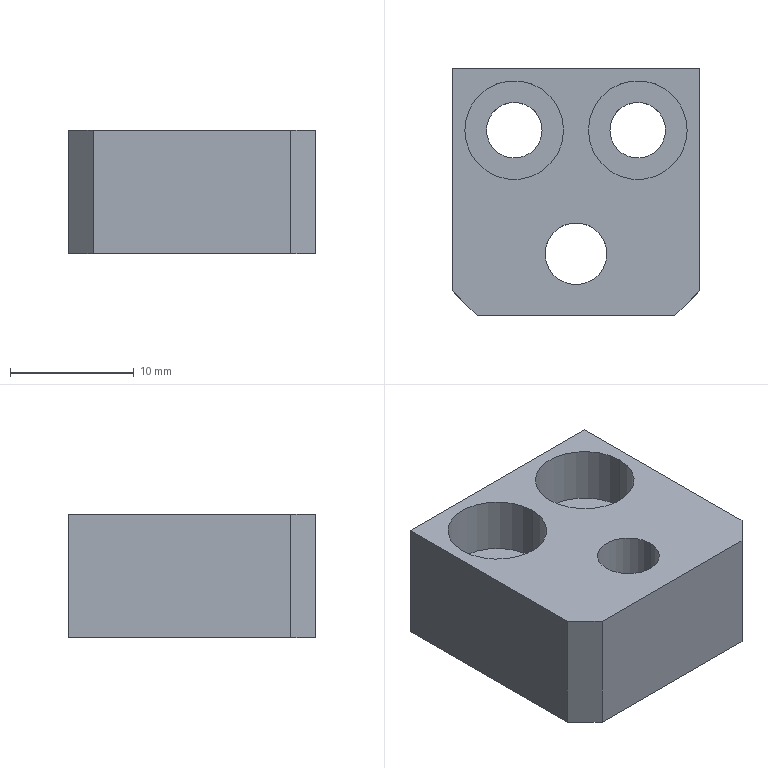Part | STEP file | 2051 Bag feed stopper block B | 1 solid | 20 faces | box 20 x 20 x 10 mm | volume 3129 mm3 | cylinder 10 | plane 10 | commonest cylinder face diameters 4.5 x4 8 x4 5 x2
STEP:
#1=CARTESIAN_POINT('',(0.,0.,0.));
#2=DIRECTION('',(0.,0.,1.));
#3=DIRECTION('',(1.,0.,0.));
#4=AXIS2_PLACEMENT_3D('',#1,#2,#3);
#5=CARTESIAN_POINT('',(2.5,-5.,0.));
#6=VERTEX_POINT('',#5);
#7=CARTESIAN_POINT('',(2.5,-5.,10.));
#8=VERTEX_POINT('',#7);
#9=CARTESIAN_POINT('',(2.5,-5.,10.));
#10=DIRECTION('',(0.,0.,1.));
#11=VECTOR('',#10,1.);
#12=LINE('',#9,#11);
#13=CARTESIAN_POINT('',(0.,-5.,10.));
#14=DIRECTION('',(0.,0.,1.));
#15=DIRECTION('',(1.,0.,0.));
#16=AXIS2_PLACEMENT_3D('',#13,#14,#15);
#17=CYLINDRICAL_SURFACE('',#16,2.5);
#18=CARTESIAN_POINT('',(6.283,0.));
#19=DIRECTION('',(0.,1.));
#20=VECTOR('',#19,1.);
#21=LINE('',#18,#20);
#22=(GEOMETRIC_REPRESENTATION_CONTEXT(2)PARAMETRIC_REPRESENTATION_CONTEXT()REPRESENTATION_CONTEXT('',''));
#23=DEFINITIONAL_REPRESENTATION('',(#21),#22);
#24=PCURVE('',#17,#23);
#25=CARTESIAN_POINT('',(0.,-5.,10.));
#26=DIRECTION('',(0.,0.,1.));
#27=DIRECTION('',(1.,0.,0.));
#28=AXIS2_PLACEMENT_3D('',#25,#26,#27);
#29=CYLINDRICAL_SURFACE('',#28,2.5);
#30=CARTESIAN_POINT('',(0.,0.));
#31=DIRECTION('',(0.,1.));
#32=VECTOR('',#31,1.);
#33=LINE('',#30,#32);
#34=(GEOMETRIC_REPRESENTATION_CONTEXT(2)PARAMETRIC_REPRESENTATION_CONTEXT()REPRESENTATION_CONTEXT('',''));
#35=DEFINITIONAL_REPRESENTATION('',(#33),#34);
#36=PCURVE('',#29,#35);
#37=SURFACE_CURVE('',#12,(#24,#36),.PCURVE_S1.);
#38=EDGE_CURVE('',#6,#8,#37,.T.);
#39=ORIENTED_EDGE('',*,*,#38,.T.);
#40=CARTESIAN_POINT('',(-2.5,-5.,10.));
#41=VERTEX_POINT('',#40);
#42=CARTESIAN_POINT('',(0.,-5.,10.));
#43=DIRECTION('',(0.,0.,1.));
#44=DIRECTION('',(1.,0.,0.));
#45=AXIS2_PLACEMENT_3D('',#42,#43,#44);
#46=CIRCLE('',#45,2.5);
#47=CARTESIAN_POINT('',(0.,0.));
#48=DIRECTION('',(1.,0.));
#49=VECTOR('',#48,1.);
#50=LINE('',#47,#49);
#51=(GEOMETRIC_REPRESENTATION_CONTEXT(2)PARAMETRIC_REPRESENTATION_CONTEXT()REPRESENTATION_CONTEXT('',''));
#52=DEFINITIONAL_REPRESENTATION('',(#50),#51);
#53=PCURVE('',#17,#52);
#54=CARTESIAN_POINT('',(0.,0.,10.));
#55=DIRECTION('',(0.,0.,-1.));
#56=DIRECTION('',(-1.,0.,0.));
#57=AXIS2_PLACEMENT_3D('',#54,#55,#56);
#58=PLANE('',#57);
#59=CARTESIAN_POINT('',(-2.5,-5.));
#60=CARTESIAN_POINT('',(-2.5,-0.6699));
#61=CARTESIAN_POINT('',(1.25,-2.835));
#62=CARTESIAN_POINT('',(5.,-5.));
#63=CARTESIAN_POINT('',(1.25,-7.165));
#64=CARTESIAN_POINT('',(-2.5,-9.33));
#65=CARTESIAN_POINT('',(-2.5,-5.));
#66=(BOUNDED_CURVE()B_SPLINE_CURVE(2,(#59,#60,#61,#62,#63,#64,#65),.UNSPECIFIED.,.T.,.F.)B_SPLINE_CURVE_WITH_KNOTS((1,2,2,2,2,1),(-2.094,0.,2.094,4.189,6.283,8.378),.UNSPECIFIED.)CURVE()GEOMETRIC_REPRESENTATION_ITEM()RATIONAL_B_SPLINE_CURVE((1.,0.5,1.,0.5,1.,0.5,1.))REPRESENTATION_ITEM(''));
#67=(GEOMETRIC_REPRESENTATION_CONTEXT(2)PARAMETRIC_REPRESENTATION_CONTEXT()REPRESENTATION_CONTEXT('',''));
#68=DEFINITIONAL_REPRESENTATION('',(#66),#67);
#69=PCURVE('',#58,#68);
#70=SURFACE_CURVE('',#46,(#53,#69),.PCURVE_S1.);
#71=EDGE_CURVE('',#41,#8,#70,.T.);
#72=ORIENTED_EDGE('',*,*,#71,.F.);
#73=CARTESIAN_POINT('',(-2.5,-5.,0.));
#74=VERTEX_POINT('',#73);
#75=CARTESIAN_POINT('',(-2.5,-5.,10.));
#76=DIRECTION('',(0.,0.,1.));
#77=VECTOR('',#76,1.);
#78=LINE('',#75,#77);
#79=CARTESIAN_POINT('',(3.142,0.));
#80=DIRECTION('',(0.,1.));
#81=VECTOR('',#80,1.);
#82=LINE('',#79,#81);
#83=(GEOMETRIC_REPRESENTATION_CONTEXT(2)PARAMETRIC_REPRESENTATION_CONTEXT()REPRESENTATION_CONTEXT('',''));
#84=DEFINITIONAL_REPRESENTATION('',(#82),#83);
#85=PCURVE('',#17,#84);
#86=CARTESIAN_POINT('',(3.142,0.));
#87=DIRECTION('',(0.,1.));
#88=VECTOR('',#87,1.);
#89=LINE('',#86,#88);
#90=(GEOMETRIC_REPRESENTATION_CONTEXT(2)PARAMETRIC_REPRESENTATION_CONTEXT()REPRESENTATION_CONTEXT('',''));
#91=DEFINITIONAL_REPRESENTATION('',(#89),#90);
#92=PCURVE('',#29,#91);
#93=SURFACE_CURVE('',#78,(#85,#92),.PCURVE_S1.);
#94=EDGE_CURVE('',#74,#41,#93,.T.);
#95=ORIENTED_EDGE('',*,*,#94,.F.);
#96=CARTESIAN_POINT('',(0.,-5.,0.));
#97=DIRECTION('',(0.,0.,-1.));
#98=DIRECTION('',(-1.,0.,0.));
#99=AXIS2_PLACEMENT_3D('',#96,#97,#98);
#100=CIRCLE('',#99,2.5);
#101=CARTESIAN_POINT('',(9.425,-10.));
#102=DIRECTION('',(-1.,0.));
#103=VECTOR('',#102,1.);
#104=LINE('',#101,#103);
#105=(GEOMETRIC_REPRESENTATION_CONTEXT(2)PARAMETRIC_REPRESENTATION_CONTEXT()REPRESENTATION_CONTEXT('',''));
#106=DEFINITIONAL_REPRESENTATION('',(#104),#105);
#107=PCURVE('',#17,#106);
#108=CARTESIAN_POINT('',(0.,0.,0.));
#109=DIRECTION('',(0.,0.,-1.));
#110=DIRECTION('',(-1.,0.,0.));
#111=AXIS2_PLACEMENT_3D('',#108,#109,#110);
#112=PLANE('',#111);
#113=CARTESIAN_POINT('',(0.,-5.));
#114=DIRECTION('',(1.,0.));
#115=AXIS2_PLACEMENT_2D('',#113,#114);
#116=CIRCLE('',#115,2.5);
#117=(GEOMETRIC_REPRESENTATION_CONTEXT(2)PARAMETRIC_REPRESENTATION_CONTEXT()REPRESENTATION_CONTEXT('',''));
#118=DEFINITIONAL_REPRESENTATION('',(#116),#117);
#119=PCURVE('',#112,#118);
#120=SURFACE_CURVE('',#100,(#107,#119),.PCURVE_S1.);
#121=EDGE_CURVE('',#6,#74,#120,.T.);
#122=ORIENTED_EDGE('',*,*,#121,.F.);
#123=EDGE_LOOP('',(#39,#72,#95,#122));
#124=FACE_BOUND('',#123,.F.);
#125=ADVANCED_FACE('',(#124),#17,.F.);
#126=CARTESIAN_POINT('',(-1.,5.,5.4));
#127=VERTEX_POINT('',#126);
#128=CARTESIAN_POINT('',(-1.,5.,10.));
#129=VERTEX_POINT('',#128);
#130=CARTESIAN_POINT('',(-1.,5.,10.));
#131=DIRECTION('',(0.,0.,1.));
#132=VECTOR('',#131,1.);
#133=LINE('',#130,#132);
#134=CARTESIAN_POINT('',(-5.,5.,10.));
#135=DIRECTION('',(0.,0.,1.));
#136=DIRECTION('',(1.,0.,0.));
#137=AXIS2_PLACEMENT_3D('',#134,#135,#136);
#138=CYLINDRICAL_SURFACE('',#137,4.);
#139=CARTESIAN_POINT('',(6.283,0.));
#140=DIRECTION('',(0.,1.));
#141=VECTOR('',#140,1.);
#142=LINE('',#139,#141);
#143=(GEOMETRIC_REPRESENTATION_CONTEXT(2)PARAMETRIC_REPRESENTATION_CONTEXT()REPRESENTATION_CONTEXT('',''));
#144=DEFINITIONAL_REPRESENTATION('',(#142),#143);
#145=PCURVE('',#138,#144);
#146=CARTESIAN_POINT('',(-5.,5.,10.));
#147=DIRECTION('',(0.,0.,1.));
#148=DIRECTION('',(1.,0.,0.));
#149=AXIS2_PLACEMENT_3D('',#146,#147,#148);
#150=CYLINDRICAL_SURFACE('',#149,4.);
#151=CARTESIAN_POINT('',(0.,0.));
#152=DIRECTION('',(0.,1.));
#153=VECTOR('',#152,1.);
#154=LINE('',#151,#153);
#155=(GEOMETRIC_REPRESENTATION_CONTEXT(2)PARAMETRIC_REPRESENTATION_CONTEXT()REPRESENTATION_CONTEXT('',''));
#156=DEFINITIONAL_REPRESENTATION('',(#154),#155);
#157=PCURVE('',#150,#156);
#158=SURFACE_CURVE('',#133,(#145,#157),.PCURVE_S1.);
#159=EDGE_CURVE('',#127,#129,#158,.T.);
#160=ORIENTED_EDGE('',*,*,#159,.T.);
#161=CARTESIAN_POINT('',(-9.,5.,10.));
#162=VERTEX_POINT('',#161);
#163=CARTESIAN_POINT('',(-5.,5.,10.));
#164=DIRECTION('',(0.,0.,1.));
#165=DIRECTION('',(1.,0.,0.));
#166=AXIS2_PLACEMENT_3D('',#163,#164,#165);
#167=CIRCLE('',#166,4.);
#168=CARTESIAN_POINT('',(0.,0.));
#169=DIRECTION('',(1.,0.));
#170=VECTOR('',#169,1.);
#171=LINE('',#168,#170);
#172=(GEOMETRIC_REPRESENTATION_CONTEXT(2)PARAMETRIC_REPRESENTATION_CONTEXT()REPRESENTATION_CONTEXT('',''));
#173=DEFINITIONAL_REPRESENTATION('',(#171),#172);
#174=PCURVE('',#138,#173);
#175=CARTESIAN_POINT('',(1.,5.));
#176=CARTESIAN_POINT('',(1.,11.928));
#177=CARTESIAN_POINT('',(7.,8.464));
#178=CARTESIAN_POINT('',(13.,5.));
#179=CARTESIAN_POINT('',(7.,1.536));
#180=CARTESIAN_POINT('',(1.,-1.928));
#181=CARTESIAN_POINT('',(1.,5.));
#182=(BOUNDED_CURVE()B_SPLINE_CURVE(2,(#175,#176,#177,#178,#179,#180,#181),.UNSPECIFIED.,.T.,.F.)B_SPLINE_CURVE_WITH_KNOTS((1,2,2,2,2,1),(-2.094,0.,2.094,4.189,6.283,8.378),.UNSPECIFIED.)CURVE()GEOMETRIC_REPRESENTATION_ITEM()RATIONAL_B_SPLINE_CURVE((1.,0.5,1.,0.5,1.,0.5,1.))REPRESENTATION_ITEM(''));
#183=(GEOMETRIC_REPRESENTATION_CONTEXT(2)PARAMETRIC_REPRESENTATION_CONTEXT()REPRESENTATION_CONTEXT('',''));
#184=DEFINITIONAL_REPRESENTATION('',(#182),#183);
#185=PCURVE('',#58,#184);
#186=SURFACE_CURVE('',#167,(#174,#185),.PCURVE_S1.);
#187=EDGE_CURVE('',#162,#129,#186,.T.);
#188=ORIENTED_EDGE('',*,*,#187,.F.);
#189=CARTESIAN_POINT('',(-9.,5.,5.4));
#190=VERTEX_POINT('',#189);
#191=CARTESIAN_POINT('',(-9.,5.,10.));
#192=DIRECTION('',(0.,0.,1.));
#193=VECTOR('',#192,1.);
#194=LINE('',#191,#193);
#195=CARTESIAN_POINT('',(3.142,0.));
#196=DIRECTION('',(0.,1.));
#197=VECTOR('',#196,1.);
#198=LINE('',#195,#197);
#199=(GEOMETRIC_REPRESENTATION_CONTEXT(2)PARAMETRIC_REPRESENTATION_CONTEXT()REPRESENTATION_CONTEXT('',''));
#200=DEFINITIONAL_REPRESENTATION('',(#198),#199);
#201=PCURVE('',#138,#200);
#202=CARTESIAN_POINT('',(3.142,0.));
#203=DIRECTION('',(0.,1.));
#204=VECTOR('',#203,1.);
#205=LINE('',#202,#204);
#206=(GEOMETRIC_REPRESENTATION_CONTEXT(2)PARAMETRIC_REPRESENTATION_CONTEXT()REPRESENTATION_CONTEXT('',''));
#207=DEFINITIONAL_REPRESENTATION('',(#205),#206);
#208=PCURVE('',#150,#207);
#209=SURFACE_CURVE('',#194,(#201,#208),.PCURVE_S1.);
#210=EDGE_CURVE('',#190,#162,#209,.T.);
#211=ORIENTED_EDGE('',*,*,#210,.F.);
#212=CARTESIAN_POINT('',(-5.,5.,5.4));
#213=DIRECTION('',(0.,0.,1.));
#214=DIRECTION('',(1.,0.,0.));
#215=AXIS2_PLACEMENT_3D('',#212,#213,#214);
#216=CIRCLE('',#215,4.);
#217=CARTESIAN_POINT('',(0.,-4.6));
#218=DIRECTION('',(1.,0.));
#219=VECTOR('',#218,1.);
#220=LINE('',#217,#219);
#221=(GEOMETRIC_REPRESENTATION_CONTEXT(2)PARAMETRIC_REPRESENTATION_CONTEXT()REPRESENTATION_CONTEXT('',''));
#222=DEFINITIONAL_REPRESENTATION('',(#220),#221);
#223=PCURVE('',#138,#222);
#224=CARTESIAN_POINT('',(-2.75,5.,5.4));
#225=DIRECTION('',(0.,0.,-1.));
#226=DIRECTION('',(-1.,0.,0.));
#227=AXIS2_PLACEMENT_3D('',#224,#225,#226);
#228=PLANE('',#227);
#229=CARTESIAN_POINT('',(-1.75,0.));
#230=CARTESIAN_POINT('',(-1.75,6.928));
#231=CARTESIAN_POINT('',(4.25,3.464));
#232=CARTESIAN_POINT('',(10.25,0.));
#233=CARTESIAN_POINT('',(4.25,-3.464));
#234=CARTESIAN_POINT('',(-1.75,-6.928));
#235=CARTESIAN_POINT('',(-1.75,0.));
#236=(BOUNDED_CURVE()B_SPLINE_CURVE(2,(#229,#230,#231,#232,#233,#234,#235),.UNSPECIFIED.,.T.,.F.)B_SPLINE_CURVE_WITH_KNOTS((1,2,2,2,2,1),(-2.094,0.,2.094,4.189,6.283,8.378),.UNSPECIFIED.)CURVE()GEOMETRIC_REPRESENTATION_ITEM()RATIONAL_B_SPLINE_CURVE((1.,0.5,1.,0.5,1.,0.5,1.))REPRESENTATION_ITEM(''));
#237=(GEOMETRIC_REPRESENTATION_CONTEXT(2)PARAMETRIC_REPRESENTATION_CONTEXT()REPRESENTATION_CONTEXT('',''));
#238=DEFINITIONAL_REPRESENTATION('',(#236),#237);
#239=PCURVE('',#228,#238);
#240=SURFACE_CURVE('',#216,(#223,#239),.PCURVE_S1.);
#241=EDGE_CURVE('',#190,#127,#240,.T.);
#242=ORIENTED_EDGE('',*,*,#241,.T.);
#243=EDGE_LOOP('',(#160,#188,#211,#242));
#244=FACE_BOUND('',#243,.F.);
#245=ADVANCED_FACE('',(#244),#138,.F.);
#246=CARTESIAN_POINT('',(-2.75,5.,0.));
#247=VERTEX_POINT('',#246);
#248=CARTESIAN_POINT('',(-2.75,5.,5.4));
#249=VERTEX_POINT('',#248);
#250=CARTESIAN_POINT('',(-2.75,5.,10.));
#251=DIRECTION('',(0.,0.,1.));
#252=VECTOR('',#251,1.);
#253=LINE('',#250,#252);
#254=CARTESIAN_POINT('',(-5.,5.,10.));
#255=DIRECTION('',(0.,0.,1.));
#256=DIRECTION('',(1.,0.,0.));
#257=AXIS2_PLACEMENT_3D('',#254,#255,#256);
#258=CYLINDRICAL_SURFACE('',#257,2.25);
#259=CARTESIAN_POINT('',(6.283,0.));
#260=DIRECTION('',(0.,1.));
#261=VECTOR('',#260,1.);
#262=LINE('',#259,#261);
#263=(GEOMETRIC_REPRESENTATION_CONTEXT(2)PARAMETRIC_REPRESENTATION_CONTEXT()REPRESENTATION_CONTEXT('',''));
#264=DEFINITIONAL_REPRESENTATION('',(#262),#263);
#265=PCURVE('',#258,#264);
#266=CARTESIAN_POINT('',(-5.,5.,10.));
#267=DIRECTION('',(0.,0.,1.));
#268=DIRECTION('',(1.,0.,0.));
#269=AXIS2_PLACEMENT_3D('',#266,#267,#268);
#270=CYLINDRICAL_SURFACE('',#269,2.25);
#271=CARTESIAN_POINT('',(0.,0.));
#272=DIRECTION('',(0.,1.));
#273=VECTOR('',#272,1.);
#274=LINE('',#271,#273);
#275=(GEOMETRIC_REPRESENTATION_CONTEXT(2)PARAMETRIC_REPRESENTATION_CONTEXT()REPRESENTATION_CONTEXT('',''));
#276=DEFINITIONAL_REPRESENTATION('',(#274),#275);
#277=PCURVE('',#270,#276);
#278=SURFACE_CURVE('',#253,(#265,#277),.PCURVE_S1.);
#279=EDGE_CURVE('',#247,#249,#278,.T.);
#280=ORIENTED_EDGE('',*,*,#279,.T.);
#281=CARTESIAN_POINT('',(-7.25,5.,5.4));
#282=VERTEX_POINT('',#281);
#283=CARTESIAN_POINT('',(-5.,5.,5.4));
#284=DIRECTION('',(0.,0.,1.));
#285=DIRECTION('',(1.,0.,0.));
#286=AXIS2_PLACEMENT_3D('',#283,#284,#285);
#287=CIRCLE('',#286,2.25);
#288=CARTESIAN_POINT('',(0.,-4.6));
#289=DIRECTION('',(1.,0.));
#290=VECTOR('',#289,1.);
#291=LINE('',#288,#290);
#292=(GEOMETRIC_REPRESENTATION_CONTEXT(2)PARAMETRIC_REPRESENTATION_CONTEXT()REPRESENTATION_CONTEXT('',''));
#293=DEFINITIONAL_REPRESENTATION('',(#291),#292);
#294=PCURVE('',#258,#293);
#295=CARTESIAN_POINT('',(0.,0.));
#296=CARTESIAN_POINT('',(0.,3.897));
#297=CARTESIAN_POINT('',(3.375,1.949));
#298=CARTESIAN_POINT('',(6.75,0.));
#299=CARTESIAN_POINT('',(3.375,-1.949));
#300=CARTESIAN_POINT('',(0.,-3.897));
#301=CARTESIAN_POINT('',(0.,0.));
#302=(BOUNDED_CURVE()B_SPLINE_CURVE(2,(#295,#296,#297,#298,#299,#300,#301),.UNSPECIFIED.,.T.,.F.)B_SPLINE_CURVE_WITH_KNOTS((1,2,2,2,2,1),(-2.094,0.,2.094,4.189,6.283,8.378),.UNSPECIFIED.)CURVE()GEOMETRIC_REPRESENTATION_ITEM()RATIONAL_B_SPLINE_CURVE((1.,0.5,1.,0.5,1.,0.5,1.))REPRESENTATION_ITEM(''));
#303=(GEOMETRIC_REPRESENTATION_CONTEXT(2)PARAMETRIC_REPRESENTATION_CONTEXT()REPRESENTATION_CONTEXT('',''));
#304=DEFINITIONAL_REPRESENTATION('',(#302),#303);
#305=PCURVE('',#228,#304);
#306=SURFACE_CURVE('',#287,(#294,#305),.PCURVE_S1.);
#307=EDGE_CURVE('',#282,#249,#306,.T.);
#308=ORIENTED_EDGE('',*,*,#307,.F.);
#309=CARTESIAN_POINT('',(-7.25,5.,0.));
#310=VERTEX_POINT('',#309);
#311=CARTESIAN_POINT('',(-7.25,5.,10.));
#312=DIRECTION('',(0.,0.,1.));
#313=VECTOR('',#312,1.);
#314=LINE('',#311,#313);
#315=CARTESIAN_POINT('',(3.142,0.));
#316=DIRECTION('',(0.,1.));
#317=VECTOR('',#316,1.);
#318=LINE('',#315,#317);
#319=(GEOMETRIC_REPRESENTATION_CONTEXT(2)PARAMETRIC_REPRESENTATION_CONTEXT()REPRESENTATION_CONTEXT('',''));
#320=DEFINITIONAL_REPRESENTATION('',(#318),#319);
#321=PCURVE('',#258,#320);
#322=CARTESIAN_POINT('',(3.142,0.));
#323=DIRECTION('',(0.,1.));
#324=VECTOR('',#323,1.);
#325=LINE('',#322,#324);
#326=(GEOMETRIC_REPRESENTATION_CONTEXT(2)PARAMETRIC_REPRESENTATION_CONTEXT()REPRESENTATION_CONTEXT('',''));
#327=DEFINITIONAL_REPRESENTATION('',(#325),#326);
#328=PCURVE('',#270,#327);
#329=SURFACE_CURVE('',#314,(#321,#328),.PCURVE_S1.);
#330=EDGE_CURVE('',#310,#282,#329,.T.);
#331=ORIENTED_EDGE('',*,*,#330,.F.);
#332=CARTESIAN_POINT('',(-5.,5.,0.));
#333=DIRECTION('',(0.,0.,-1.));
#334=DIRECTION('',(-1.,0.,0.));
#335=AXIS2_PLACEMENT_3D('',#332,#333,#334);
#336=CIRCLE('',#335,2.25);
#337=CARTESIAN_POINT('',(9.425,-10.));
#338=DIRECTION('',(-1.,0.));
#339=VECTOR('',#338,1.);
#340=LINE('',#337,#339);
#341=(GEOMETRIC_REPRESENTATION_CONTEXT(2)PARAMETRIC_REPRESENTATION_CONTEXT()REPRESENTATION_CONTEXT('',''));
#342=DEFINITIONAL_REPRESENTATION('',(#340),#341);
#343=PCURVE('',#258,#342);
#344=CARTESIAN_POINT('',(5.,5.));
#345=DIRECTION('',(1.,0.));
#346=AXIS2_PLACEMENT_2D('',#344,#345);
#347=CIRCLE('',#346,2.25);
#348=(GEOMETRIC_REPRESENTATION_CONTEXT(2)PARAMETRIC_REPRESENTATION_CONTEXT()REPRESENTATION_CONTEXT('',''));
#349=DEFINITIONAL_REPRESENTATION('',(#347),#348);
#350=PCURVE('',#112,#349);
#351=SURFACE_CURVE('',#336,(#343,#350),.PCURVE_S1.);
#352=EDGE_CURVE('',#247,#310,#351,.T.);
#353=ORIENTED_EDGE('',*,*,#352,.F.);
#354=EDGE_LOOP('',(#280,#308,#331,#353));
#355=FACE_BOUND('',#354,.F.);
#356=ADVANCED_FACE('',(#355),#258,.F.);
#357=CARTESIAN_POINT('',(9.,5.,5.4));
#358=VERTEX_POINT('',#357);
#359=CARTESIAN_POINT('',(9.,5.,10.));
#360=VERTEX_POINT('',#359);
#361=CARTESIAN_POINT('',(9.,5.,10.));
#362=DIRECTION('',(0.,0.,1.));
#363=VECTOR('',#362,1.);
#364=LINE('',#361,#363);
#365=CARTESIAN_POINT('',(5.,5.,10.));
#366=DIRECTION('',(0.,0.,1.));
#367=DIRECTION('',(1.,0.,0.));
#368=AXIS2_PLACEMENT_3D('',#365,#366,#367);
#369=CYLINDRICAL_SURFACE('',#368,4.);
#370=CARTESIAN_POINT('',(6.283,0.));
#371=DIRECTION('',(0.,1.));
#372=VECTOR('',#371,1.);
#373=LINE('',#370,#372);
#374=(GEOMETRIC_REPRESENTATION_CONTEXT(2)PARAMETRIC_REPRESENTATION_CONTEXT()REPRESENTATION_CONTEXT('',''));
#375=DEFINITIONAL_REPRESENTATION('',(#373),#374);
#376=PCURVE('',#369,#375);
#377=CARTESIAN_POINT('',(5.,5.,10.));
#378=DIRECTION('',(0.,0.,1.));
#379=DIRECTION('',(1.,0.,0.));
#380=AXIS2_PLACEMENT_3D('',#377,#378,#379);
#381=CYLINDRICAL_SURFACE('',#380,4.);
#382=CARTESIAN_POINT('',(0.,0.));
#383=DIRECTION('',(0.,1.));
#384=VECTOR('',#383,1.);
#385=LINE('',#382,#384);
#386=(GEOMETRIC_REPRESENTATION_CONTEXT(2)PARAMETRIC_REPRESENTATION_CONTEXT()REPRESENTATION_CONTEXT('',''));
#387=DEFINITIONAL_REPRESENTATION('',(#385),#386);
#388=PCURVE('',#381,#387);
#389=SURFACE_CURVE('',#364,(#376,#388),.PCURVE_S1.);
#390=EDGE_CURVE('',#358,#360,#389,.T.);
#391=ORIENTED_EDGE('',*,*,#390,.T.);
#392=CARTESIAN_POINT('',(1.,5.,10.));
#393=VERTEX_POINT('',#392);
#394=CARTESIAN_POINT('',(5.,5.,10.));
#395=DIRECTION('',(0.,0.,1.));
#396=DIRECTION('',(1.,0.,0.));
#397=AXIS2_PLACEMENT_3D('',#394,#395,#396);
#398=CIRCLE('',#397,4.);
#399=CARTESIAN_POINT('',(0.,0.));
#400=DIRECTION('',(1.,0.));
#401=VECTOR('',#400,1.);
#402=LINE('',#399,#401);
#403=(GEOMETRIC_REPRESENTATION_CONTEXT(2)PARAMETRIC_REPRESENTATION_CONTEXT()REPRESENTATION_CONTEXT('',''));
#404=DEFINITIONAL_REPRESENTATION('',(#402),#403);
#405=PCURVE('',#369,#404);
#406=CARTESIAN_POINT('',(-9.,5.));
#407=CARTESIAN_POINT('',(-9.,11.928));
#408=CARTESIAN_POINT('',(-3.,8.464));
#409=CARTESIAN_POINT('',(3.,5.));
#410=CARTESIAN_POINT('',(-3.,1.536));
#411=CARTESIAN_POINT('',(-9.,-1.928));
#412=CARTESIAN_POINT('',(-9.,5.));
#413=(BOUNDED_CURVE()B_SPLINE_CURVE(2,(#406,#407,#408,#409,#410,#411,#412),.UNSPECIFIED.,.T.,.F.)B_SPLINE_CURVE_WITH_KNOTS((1,2,2,2,2,1),(-2.094,0.,2.094,4.189,6.283,8.378),.UNSPECIFIED.)CURVE()GEOMETRIC_REPRESENTATION_ITEM()RATIONAL_B_SPLINE_CURVE((1.,0.5,1.,0.5,1.,0.5,1.))REPRESENTATION_ITEM(''));
#414=(GEOMETRIC_REPRESENTATION_CONTEXT(2)PARAMETRIC_REPRESENTATION_CONTEXT()REPRESENTATION_CONTEXT('',''));
#415=DEFINITIONAL_REPRESENTATION('',(#413),#414);
#416=PCURVE('',#58,#415);
#417=SURFACE_CURVE('',#398,(#405,#416),.PCURVE_S1.);
#418=EDGE_CURVE('',#393,#360,#417,.T.);
#419=ORIENTED_EDGE('',*,*,#418,.F.);
#420=CARTESIAN_POINT('',(1.,5.,5.4));
#421=VERTEX_POINT('',#420);
#422=CARTESIAN_POINT('',(1.,5.,10.));
#423=DIRECTION('',(0.,0.,1.));
#424=VECTOR('',#423,1.);
#425=LINE('',#422,#424);
#426=CARTESIAN_POINT('',(3.142,0.));
#427=DIRECTION('',(0.,1.));
#428=VECTOR('',#427,1.);
#429=LINE('',#426,#428);
#430=(GEOMETRIC_REPRESENTATION_CONTEXT(2)PARAMETRIC_REPRESENTATION_CONTEXT()REPRESENTATION_CONTEXT('',''));
#431=DEFINITIONAL_REPRESENTATION('',(#429),#430);
#432=PCURVE('',#369,#431);
#433=CARTESIAN_POINT('',(3.142,0.));
#434=DIRECTION('',(0.,1.));
#435=VECTOR('',#434,1.);
#436=LINE('',#433,#435);
#437=(GEOMETRIC_REPRESENTATION_CONTEXT(2)PARAMETRIC_REPRESENTATION_CONTEXT()REPRESENTATION_CONTEXT('',''));
#438=DEFINITIONAL_REPRESENTATION('',(#436),#437);
#439=PCURVE('',#381,#438);
#440=SURFACE_CURVE('',#425,(#432,#439),.PCURVE_S1.);
#441=EDGE_CURVE('',#421,#393,#440,.T.);
#442=ORIENTED_EDGE('',*,*,#441,.F.);
#443=CARTESIAN_POINT('',(5.,5.,5.4));
#444=DIRECTION('',(0.,0.,1.));
#445=DIRECTION('',(1.,0.,0.));
#446=AXIS2_PLACEMENT_3D('',#443,#444,#445);
#447=CIRCLE('',#446,4.);
#448=CARTESIAN_POINT('',(0.,-4.6));
#449=DIRECTION('',(1.,0.));
#450=VECTOR('',#449,1.);
#451=LINE('',#448,#450);
#452=(GEOMETRIC_REPRESENTATION_CONTEXT(2)PARAMETRIC_REPRESENTATION_CONTEXT()REPRESENTATION_CONTEXT('',''));
#453=DEFINITIONAL_REPRESENTATION('',(#451),#452);
#454=PCURVE('',#369,#453);
#455=CARTESIAN_POINT('',(7.25,5.,5.4));
#456=DIRECTION('',(0.,0.,-1.));
#457=DIRECTION('',(-1.,0.,0.));
#458=AXIS2_PLACEMENT_3D('',#455,#456,#457);
#459=PLANE('',#458);
#460=CARTESIAN_POINT('',(-1.75,0.));
#461=CARTESIAN_POINT('',(-1.75,6.928));
#462=CARTESIAN_POINT('',(4.25,3.464));
#463=CARTESIAN_POINT('',(10.25,0.));
#464=CARTESIAN_POINT('',(4.25,-3.464));
#465=CARTESIAN_POINT('',(-1.75,-6.928));
#466=CARTESIAN_POINT('',(-1.75,0.));
#467=(BOUNDED_CURVE()B_SPLINE_CURVE(2,(#460,#461,#462,#463,#464,#465,#466),.UNSPECIFIED.,.T.,.F.)B_SPLINE_CURVE_WITH_KNOTS((1,2,2,2,2,1),(-2.094,0.,2.094,4.189,6.283,8.378),.UNSPECIFIED.)CURVE()GEOMETRIC_REPRESENTATION_ITEM()RATIONAL_B_SPLINE_CURVE((1.,0.5,1.,0.5,1.,0.5,1.))REPRESENTATION_ITEM(''));
#468=(GEOMETRIC_REPRESENTATION_CONTEXT(2)PARAMETRIC_REPRESENTATION_CONTEXT()REPRESENTATION_CONTEXT('',''));
#469=DEFINITIONAL_REPRESENTATION('',(#467),#468);
#470=PCURVE('',#459,#469);
#471=SURFACE_CURVE('',#447,(#454,#470),.PCURVE_S1.);
#472=EDGE_CURVE('',#421,#358,#471,.T.);
#473=ORIENTED_EDGE('',*,*,#472,.T.);
#474=EDGE_LOOP('',(#391,#419,#442,#473));
#475=FACE_BOUND('',#474,.F.);
#476=ADVANCED_FACE('',(#475),#369,.F.);
#477=CARTESIAN_POINT('',(7.25,5.,0.));
#478=VERTEX_POINT('',#477);
#479=CARTESIAN_POINT('',(7.25,5.,5.4));
#480=VERTEX_POINT('',#479);
#481=CARTESIAN_POINT('',(7.25,5.,10.));
#482=DIRECTION('',(0.,0.,1.));
#483=VECTOR('',#482,1.);
#484=LINE('',#481,#483);
#485=CARTESIAN_POINT('',(5.,5.,10.));
#486=DIRECTION('',(0.,0.,1.));
#487=DIRECTION('',(1.,0.,0.));
#488=AXIS2_PLACEMENT_3D('',#485,#486,#487);
#489=CYLINDRICAL_SURFACE('',#488,2.25);
#490=CARTESIAN_POINT('',(6.283,0.));
#491=DIRECTION('',(0.,1.));
#492=VECTOR('',#491,1.);
#493=LINE('',#490,#492);
#494=(GEOMETRIC_REPRESENTATION_CONTEXT(2)PARAMETRIC_REPRESENTATION_CONTEXT()REPRESENTATION_CONTEXT('',''));
#495=DEFINITIONAL_REPRESENTATION('',(#493),#494);
#496=PCURVE('',#489,#495);
#497=CARTESIAN_POINT('',(5.,5.,10.));
#498=DIRECTION('',(0.,0.,1.));
#499=DIRECTION('',(1.,0.,0.));
#500=AXIS2_PLACEMENT_3D('',#497,#498,#499);
#501=CYLINDRICAL_SURFACE('',#500,2.25);
#502=CARTESIAN_POINT('',(0.,0.));
#503=DIRECTION('',(0.,1.));
#504=VECTOR('',#503,1.);
#505=LINE('',#502,#504);
#506=(GEOMETRIC_REPRESENTATION_CONTEXT(2)PARAMETRIC_REPRESENTATION_CONTEXT()REPRESENTATION_CONTEXT('',''));
#507=DEFINITIONAL_REPRESENTATION('',(#505),#506);
#508=PCURVE('',#501,#507);
#509=SURFACE_CURVE('',#484,(#496,#508),.PCURVE_S1.);
#510=EDGE_CURVE('',#478,#480,#509,.T.);
#511=ORIENTED_EDGE('',*,*,#510,.T.);
#512=CARTESIAN_POINT('',(2.75,5.,5.4));
#513=VERTEX_POINT('',#512);
#514=CARTESIAN_POINT('',(5.,5.,5.4));
#515=DIRECTION('',(0.,0.,1.));
#516=DIRECTION('',(1.,0.,0.));
#517=AXIS2_PLACEMENT_3D('',#514,#515,#516);
#518=CIRCLE('',#517,2.25);
#519=CARTESIAN_POINT('',(0.,-4.6));
#520=DIRECTION('',(1.,0.));
#521=VECTOR('',#520,1.);
#522=LINE('',#519,#521);
#523=(GEOMETRIC_REPRESENTATION_CONTEXT(2)PARAMETRIC_REPRESENTATION_CONTEXT()REPRESENTATION_CONTEXT('',''));
#524=DEFINITIONAL_REPRESENTATION('',(#522),#523);
#525=PCURVE('',#489,#524);
#526=CARTESIAN_POINT('',(0.,0.));
#527=CARTESIAN_POINT('',(0.,3.897));
#528=CARTESIAN_POINT('',(3.375,1.949));
#529=CARTESIAN_POINT('',(6.75,0.));
#530=CARTESIAN_POINT('',(3.375,-1.949));
#531=CARTESIAN_POINT('',(0.,-3.897));
#532=CARTESIAN_POINT('',(0.,0.));
#533=(BOUNDED_CURVE()B_SPLINE_CURVE(2,(#526,#527,#528,#529,#530,#531,#532),.UNSPECIFIED.,.T.,.F.)B_SPLINE_CURVE_WITH_KNOTS((1,2,2,2,2,1),(-2.094,0.,2.094,4.189,6.283,8.378),.UNSPECIFIED.)CURVE()GEOMETRIC_REPRESENTATION_ITEM()RATIONAL_B_SPLINE_CURVE((1.,0.5,1.,0.5,1.,0.5,1.))REPRESENTATION_ITEM(''));
#534=(GEOMETRIC_REPRESENTATION_CONTEXT(2)PARAMETRIC_REPRESENTATION_CONTEXT()REPRESENTATION_CONTEXT('',''));
#535=DEFINITIONAL_REPRESENTATION('',(#533),#534);
#536=PCURVE('',#459,#535);
#537=SURFACE_CURVE('',#518,(#525,#536),.PCURVE_S1.);
#538=EDGE_CURVE('',#513,#480,#537,.T.);
#539=ORIENTED_EDGE('',*,*,#538,.F.);
#540=CARTESIAN_POINT('',(2.75,5.,0.));
#541=VERTEX_POINT('',#540);
#542=CARTESIAN_POINT('',(2.75,5.,10.));
#543=DIRECTION('',(0.,0.,1.));
#544=VECTOR('',#543,1.);
#545=LINE('',#542,#544);
#546=CARTESIAN_POINT('',(3.142,0.));
#547=DIRECTION('',(0.,1.));
#548=VECTOR('',#547,1.);
#549=LINE('',#546,#548);
#550=(GEOMETRIC_REPRESENTATION_CONTEXT(2)PARAMETRIC_REPRESENTATION_CONTEXT()REPRESENTATION_CONTEXT('',''));
#551=DEFINITIONAL_REPRESENTATION('',(#549),#550);
#552=PCURVE('',#489,#551);
#553=CARTESIAN_POINT('',(3.142,0.));
#554=DIRECTION('',(0.,1.));
#555=VECTOR('',#554,1.);
#556=LINE('',#553,#555);
#557=(GEOMETRIC_REPRESENTATION_CONTEXT(2)PARAMETRIC_REPRESENTATION_CONTEXT()REPRESENTATION_CONTEXT('',''));
#558=DEFINITIONAL_REPRESENTATION('',(#556),#557);
#559=PCURVE('',#501,#558);
#560=SURFACE_CURVE('',#545,(#552,#559),.PCURVE_S1.);
#561=EDGE_CURVE('',#541,#513,#560,.T.);
#562=ORIENTED_EDGE('',*,*,#561,.F.);
#563=CARTESIAN_POINT('',(5.,5.,0.));
#564=DIRECTION('',(0.,0.,-1.));
#565=DIRECTION('',(-1.,0.,0.));
#566=AXIS2_PLACEMENT_3D('',#563,#564,#565);
#567=CIRCLE('',#566,2.25);
#568=CARTESIAN_POINT('',(9.425,-10.));
#569=DIRECTION('',(-1.,0.));
#570=VECTOR('',#569,1.);
#571=LINE('',#568,#570);
#572=(GEOMETRIC_REPRESENTATION_CONTEXT(2)PARAMETRIC_REPRESENTATION_CONTEXT()REPRESENTATION_CONTEXT('',''));
#573=DEFINITIONAL_REPRESENTATION('',(#571),#572);
#574=PCURVE('',#489,#573);
#575=CARTESIAN_POINT('',(-5.,5.));
#576=DIRECTION('',(1.,0.));
#577=AXIS2_PLACEMENT_2D('',#575,#576);
#578=CIRCLE('',#577,2.25);
#579=(GEOMETRIC_REPRESENTATION_CONTEXT(2)PARAMETRIC_REPRESENTATION_CONTEXT()REPRESENTATION_CONTEXT('',''));
#580=DEFINITIONAL_REPRESENTATION('',(#578),#579);
#581=PCURVE('',#112,#580);
#582=SURFACE_CURVE('',#567,(#574,#581),.PCURVE_S1.);
#583=EDGE_CURVE('',#478,#541,#582,.T.);
#584=ORIENTED_EDGE('',*,*,#583,.F.);
#585=EDGE_LOOP('',(#511,#539,#562,#584));
#586=FACE_BOUND('',#585,.F.);
#587=ADVANCED_FACE('',(#586),#489,.F.);
#588=CARTESIAN_POINT('',(10.,-8.,10.));
#589=VERTEX_POINT('',#588);
#590=CARTESIAN_POINT('',(10.,10.,10.));
#591=VERTEX_POINT('',#590);
#592=CARTESIAN_POINT('',(10.,-10.,10.));
#593=DIRECTION('',(0.,1.,0.));
#594=VECTOR('',#593,1.);
#595=LINE('',#592,#594);
#596=CARTESIAN_POINT('',(10.,-10.,10.));
#597=DIRECTION('',(-1.,0.,0.));
#598=DIRECTION('',(0.,0.,1.));
#599=AXIS2_PLACEMENT_3D('',#596,#597,#598);
#600=PLANE('',#599);
#601=CARTESIAN_POINT('',(0.,0.));
#602=DIRECTION('',(0.,1.));
#603=VECTOR('',#602,1.);
#604=LINE('',#601,#603);
#605=(GEOMETRIC_REPRESENTATION_CONTEXT(2)PARAMETRIC_REPRESENTATION_CONTEXT()REPRESENTATION_CONTEXT('',''));
#606=DEFINITIONAL_REPRESENTATION('',(#604),#605);
#607=PCURVE('',#600,#606);
#608=CARTESIAN_POINT('',(-10.,-10.));
#609=DIRECTION('',(0.,1.));
#610=VECTOR('',#609,1.);
#611=LINE('',#608,#610);
#612=(GEOMETRIC_REPRESENTATION_CONTEXT(2)PARAMETRIC_REPRESENTATION_CONTEXT()REPRESENTATION_CONTEXT('',''));
#613=DEFINITIONAL_REPRESENTATION('',(#611),#612);
#614=PCURVE('',#58,#613);
#615=SURFACE_CURVE('',#595,(#607,#614),.PCURVE_S1.);
#616=EDGE_CURVE('',#589,#591,#615,.T.);
#617=ORIENTED_EDGE('',*,*,#616,.F.);
#618=CARTESIAN_POINT('',(10.,-8.,0.));
#619=VERTEX_POINT('',#618);
#620=CARTESIAN_POINT('',(10.,-8.,10.));
#621=DIRECTION('',(0.,0.,-1.));
#622=VECTOR('',#621,1.);
#623=LINE('',#620,#622);
#624=CARTESIAN_POINT('',(0.,2.));
#625=DIRECTION('',(-1.,0.));
#626=VECTOR('',#625,1.);
#627=LINE('',#624,#626);
#628=(GEOMETRIC_REPRESENTATION_CONTEXT(2)PARAMETRIC_REPRESENTATION_CONTEXT()REPRESENTATION_CONTEXT('',''));
#629=DEFINITIONAL_REPRESENTATION('',(#627),#628);
#630=PCURVE('',#600,#629);
#631=CARTESIAN_POINT('',(10.,-8.,10.));
#632=DIRECTION('',(-0.7071,0.7071,0.));
#633=DIRECTION('',(0.,0.,-1.));
#634=AXIS2_PLACEMENT_3D('',#631,#632,#633);
#635=PLANE('',#634);
#636=CARTESIAN_POINT('',(0.,0.));
#637=DIRECTION('',(1.,0.));
#638=VECTOR('',#637,1.);
#639=LINE('',#636,#638);
#640=(GEOMETRIC_REPRESENTATION_CONTEXT(2)PARAMETRIC_REPRESENTATION_CONTEXT()REPRESENTATION_CONTEXT('',''));
#641=DEFINITIONAL_REPRESENTATION('',(#639),#640);
#642=PCURVE('',#635,#641);
#643=SURFACE_CURVE('',#623,(#630,#642),.PCURVE_S1.);
#644=EDGE_CURVE('',#589,#619,#643,.T.);
#645=ORIENTED_EDGE('',*,*,#644,.T.);
#646=CARTESIAN_POINT('',(10.,10.,0.));
#647=VERTEX_POINT('',#646);
#648=CARTESIAN_POINT('',(10.,-10.,0.));
#649=DIRECTION('',(0.,1.,0.));
#650=VECTOR('',#649,1.);
#651=LINE('',#648,#650);
#652=CARTESIAN_POINT('',(-10.,0.));
#653=DIRECTION('',(0.,1.));
#654=VECTOR('',#653,1.);
#655=LINE('',#652,#654);
#656=(GEOMETRIC_REPRESENTATION_CONTEXT(2)PARAMETRIC_REPRESENTATION_CONTEXT()REPRESENTATION_CONTEXT('',''));
#657=DEFINITIONAL_REPRESENTATION('',(#655),#656);
#658=PCURVE('',#600,#657);
#659=CARTESIAN_POINT('',(-10.,-10.));
#660=DIRECTION('',(0.,1.));
#661=VECTOR('',#660,1.);
#662=LINE('',#659,#661);
#663=(GEOMETRIC_REPRESENTATION_CONTEXT(2)PARAMETRIC_REPRESENTATION_CONTEXT()REPRESENTATION_CONTEXT('',''));
#664=DEFINITIONAL_REPRESENTATION('',(#662),#663);
#665=PCURVE('',#112,#664);
#666=SURFACE_CURVE('',#651,(#658,#665),.PCURVE_S1.);
#667=EDGE_CURVE('',#619,#647,#666,.T.);
#668=ORIENTED_EDGE('',*,*,#667,.T.);
#669=CARTESIAN_POINT('',(10.,10.,10.));
#670=DIRECTION('',(0.,0.,-1.));
#671=VECTOR('',#670,1.);
#672=LINE('',#669,#671);
#673=CARTESIAN_POINT('',(0.,20.));
#674=DIRECTION('',(-1.,0.));
#675=VECTOR('',#674,1.);
#676=LINE('',#673,#675);
#677=(GEOMETRIC_REPRESENTATION_CONTEXT(2)PARAMETRIC_REPRESENTATION_CONTEXT()REPRESENTATION_CONTEXT('',''));
#678=DEFINITIONAL_REPRESENTATION('',(#676),#677);
#679=PCURVE('',#600,#678);
#680=CARTESIAN_POINT('',(-10.,10.,10.));
#681=DIRECTION('',(0.,-1.,0.));
#682=DIRECTION('',(0.,0.,-1.));
#683=AXIS2_PLACEMENT_3D('',#680,#681,#682);
#684=PLANE('',#683);
#685=CARTESIAN_POINT('',(0.,20.));
#686=DIRECTION('',(1.,0.));
#687=VECTOR('',#686,1.);
#688=LINE('',#685,#687);
#689=(GEOMETRIC_REPRESENTATION_CONTEXT(2)PARAMETRIC_REPRESENTATION_CONTEXT()REPRESENTATION_CONTEXT('',''));
#690=DEFINITIONAL_REPRESENTATION('',(#688),#689);
#691=PCURVE('',#684,#690);
#692=SURFACE_CURVE('',#672,(#679,#691),.PCURVE_S1.);
#693=EDGE_CURVE('',#591,#647,#692,.T.);
#694=ORIENTED_EDGE('',*,*,#693,.F.);
#695=EDGE_LOOP('',(#617,#645,#668,#694));
#696=FACE_BOUND('',#695,.T.);
#697=ADVANCED_FACE('',(#696),#600,.F.);
#698=CARTESIAN_POINT('',(-10.,10.,0.));
#699=VERTEX_POINT('',#698);
#700=CARTESIAN_POINT('',(-10.,10.,0.));
#701=DIRECTION('',(-1.,0.,0.));
#702=VECTOR('',#701,1.);
#703=LINE('',#700,#702);
#704=CARTESIAN_POINT('',(10.,0.));
#705=DIRECTION('',(0.,-1.));
#706=VECTOR('',#705,1.);
#707=LINE('',#704,#706);
#708=(GEOMETRIC_REPRESENTATION_CONTEXT(2)PARAMETRIC_REPRESENTATION_CONTEXT()REPRESENTATION_CONTEXT('',''));
#709=DEFINITIONAL_REPRESENTATION('',(#707),#708);
#710=PCURVE('',#684,#709);
#711=CARTESIAN_POINT('',(10.,10.));
#712=DIRECTION('',(1.,0.));
#713=VECTOR('',#712,1.);
#714=LINE('',#711,#713);
#715=(GEOMETRIC_REPRESENTATION_CONTEXT(2)PARAMETRIC_REPRESENTATION_CONTEXT()REPRESENTATION_CONTEXT('',''));
#716=DEFINITIONAL_REPRESENTATION('',(#714),#715);
#717=PCURVE('',#112,#716);
#718=SURFACE_CURVE('',#703,(#710,#717),.PCURVE_S1.);
#719=EDGE_CURVE('',#647,#699,#718,.T.);
#720=ORIENTED_EDGE('',*,*,#719,.T.);
#721=CARTESIAN_POINT('',(-10.,10.,10.));
#722=VERTEX_POINT('',#721);
#723=CARTESIAN_POINT('',(-10.,10.,10.));
#724=DIRECTION('',(0.,0.,-1.));
#725=VECTOR('',#724,1.);
#726=LINE('',#723,#725);
#727=CARTESIAN_POINT('',(0.,0.));
#728=DIRECTION('',(1.,0.));
#729=VECTOR('',#728,1.);
#730=LINE('',#727,#729);
#731=(GEOMETRIC_REPRESENTATION_CONTEXT(2)PARAMETRIC_REPRESENTATION_CONTEXT()REPRESENTATION_CONTEXT('',''));
#732=DEFINITIONAL_REPRESENTATION('',(#730),#731);
#733=PCURVE('',#684,#732);
#734=CARTESIAN_POINT('',(-10.,-10.,10.));
#735=DIRECTION('',(1.,0.,0.));
#736=DIRECTION('',(0.,0.,-1.));
#737=AXIS2_PLACEMENT_3D('',#734,#735,#736);
#738=PLANE('',#737);
#739=CARTESIAN_POINT('',(0.,20.));
#740=DIRECTION('',(1.,0.));
#741=VECTOR('',#740,1.);
#742=LINE('',#739,#741);
#743=(GEOMETRIC_REPRESENTATION_CONTEXT(2)PARAMETRIC_REPRESENTATION_CONTEXT()REPRESENTATION_CONTEXT('',''));
#744=DEFINITIONAL_REPRESENTATION('',(#742),#743);
#745=PCURVE('',#738,#744);
#746=SURFACE_CURVE('',#726,(#733,#745),.PCURVE_S1.);
#747=EDGE_CURVE('',#722,#699,#746,.T.);
#748=ORIENTED_EDGE('',*,*,#747,.F.);
#749=CARTESIAN_POINT('',(-10.,10.,10.));
#750=DIRECTION('',(-1.,0.,0.));
#751=VECTOR('',#750,1.);
#752=LINE('',#749,#751);
#753=CARTESIAN_POINT('',(0.,0.));
#754=DIRECTION('',(0.,-1.));
#755=VECTOR('',#754,1.);
#756=LINE('',#753,#755);
#757=(GEOMETRIC_REPRESENTATION_CONTEXT(2)PARAMETRIC_REPRESENTATION_CONTEXT()REPRESENTATION_CONTEXT('',''));
#758=DEFINITIONAL_REPRESENTATION('',(#756),#757);
#759=PCURVE('',#684,#758);
#760=CARTESIAN_POINT('',(10.,10.));
#761=DIRECTION('',(1.,0.));
#762=VECTOR('',#761,1.);
#763=LINE('',#760,#762);
#764=(GEOMETRIC_REPRESENTATION_CONTEXT(2)PARAMETRIC_REPRESENTATION_CONTEXT()REPRESENTATION_CONTEXT('',''));
#765=DEFINITIONAL_REPRESENTATION('',(#763),#764);
#766=PCURVE('',#58,#765);
#767=SURFACE_CURVE('',#752,(#759,#766),.PCURVE_S1.);
#768=EDGE_CURVE('',#591,#722,#767,.T.);
#769=ORIENTED_EDGE('',*,*,#768,.F.);
#770=ORIENTED_EDGE('',*,*,#693,.T.);
#771=EDGE_LOOP('',(#720,#748,#769,#770));
#772=FACE_BOUND('',#771,.T.);
#773=ADVANCED_FACE('',(#772),#684,.F.);
#774=CARTESIAN_POINT('',(-10.,-8.,0.));
#775=VERTEX_POINT('',#774);
#776=CARTESIAN_POINT('',(-10.,-10.,0.));
#777=DIRECTION('',(0.,-1.,0.));
#778=VECTOR('',#777,1.);
#779=LINE('',#776,#778);
#780=CARTESIAN_POINT('',(10.,0.));
#781=DIRECTION('',(0.,-1.));
#782=VECTOR('',#781,1.);
#783=LINE('',#780,#782);
#784=(GEOMETRIC_REPRESENTATION_CONTEXT(2)PARAMETRIC_REPRESENTATION_CONTEXT()REPRESENTATION_CONTEXT('',''));
#785=DEFINITIONAL_REPRESENTATION('',(#783),#784);
#786=PCURVE('',#738,#785);
#787=CARTESIAN_POINT('',(10.,-10.));
#788=DIRECTION('',(0.,-1.));
#789=VECTOR('',#788,1.);
#790=LINE('',#787,#789);
#791=(GEOMETRIC_REPRESENTATION_CONTEXT(2)PARAMETRIC_REPRESENTATION_CONTEXT()REPRESENTATION_CONTEXT('',''));
#792=DEFINITIONAL_REPRESENTATION('',(#790),#791);
#793=PCURVE('',#112,#792);
#794=SURFACE_CURVE('',#779,(#786,#793),.PCURVE_S1.);
#795=EDGE_CURVE('',#699,#775,#794,.T.);
#796=ORIENTED_EDGE('',*,*,#795,.T.);
#797=CARTESIAN_POINT('',(-10.,-8.,10.));
#798=VERTEX_POINT('',#797);
#799=CARTESIAN_POINT('',(-10.,-8.,10.));
#800=DIRECTION('',(0.,0.,1.));
#801=VECTOR('',#800,1.);
#802=LINE('',#799,#801);
#803=CARTESIAN_POINT('',(0.,2.));
#804=DIRECTION('',(-1.,0.));
#805=VECTOR('',#804,1.);
#806=LINE('',#803,#805);
#807=(GEOMETRIC_REPRESENTATION_CONTEXT(2)PARAMETRIC_REPRESENTATION_CONTEXT()REPRESENTATION_CONTEXT('',''));
#808=DEFINITIONAL_REPRESENTATION('',(#806),#807);
#809=PCURVE('',#738,#808);
#810=CARTESIAN_POINT('',(-8.,-10.,10.));
#811=DIRECTION('',(0.7071,0.7071,0.));
#812=DIRECTION('',(0.,0.,-1.));
#813=AXIS2_PLACEMENT_3D('',#810,#811,#812);
#814=PLANE('',#813);
#815=CARTESIAN_POINT('',(0.,2.828));
#816=DIRECTION('',(-1.,0.));
#817=VECTOR('',#816,1.);
#818=LINE('',#815,#817);
#819=(GEOMETRIC_REPRESENTATION_CONTEXT(2)PARAMETRIC_REPRESENTATION_CONTEXT()REPRESENTATION_CONTEXT('',''));
#820=DEFINITIONAL_REPRESENTATION('',(#818),#819);
#821=PCURVE('',#814,#820);
#822=SURFACE_CURVE('',#802,(#809,#821),.PCURVE_S1.);
#823=EDGE_CURVE('',#775,#798,#822,.T.);
#824=ORIENTED_EDGE('',*,*,#823,.T.);
#825=CARTESIAN_POINT('',(-10.,-10.,10.));
#826=DIRECTION('',(0.,-1.,0.));
#827=VECTOR('',#826,1.);
#828=LINE('',#825,#827);
#829=CARTESIAN_POINT('',(0.,0.));
#830=DIRECTION('',(0.,-1.));
#831=VECTOR('',#830,1.);
#832=LINE('',#829,#831);
#833=(GEOMETRIC_REPRESENTATION_CONTEXT(2)PARAMETRIC_REPRESENTATION_CONTEXT()REPRESENTATION_CONTEXT('',''));
#834=DEFINITIONAL_REPRESENTATION('',(#832),#833);
#835=PCURVE('',#738,#834);
#836=CARTESIAN_POINT('',(10.,-10.));
#837=DIRECTION('',(0.,-1.));
#838=VECTOR('',#837,1.);
#839=LINE('',#836,#838);
#840=(GEOMETRIC_REPRESENTATION_CONTEXT(2)PARAMETRIC_REPRESENTATION_CONTEXT()REPRESENTATION_CONTEXT('',''));
#841=DEFINITIONAL_REPRESENTATION('',(#839),#840);
#842=PCURVE('',#58,#841);
#843=SURFACE_CURVE('',#828,(#835,#842),.PCURVE_S1.);
#844=EDGE_CURVE('',#722,#798,#843,.T.);
#845=ORIENTED_EDGE('',*,*,#844,.F.);
#846=ORIENTED_EDGE('',*,*,#747,.T.);
#847=EDGE_LOOP('',(#796,#824,#845,#846));
#848=FACE_BOUND('',#847,.T.);
#849=ADVANCED_FACE('',(#848),#738,.F.);
#850=CARTESIAN_POINT('',(-8.,-10.,0.));
#851=VERTEX_POINT('',#850);
#852=CARTESIAN_POINT('',(8.,-10.,0.));
#853=VERTEX_POINT('',#852);
#854=CARTESIAN_POINT('',(-10.,-10.,0.));
#855=DIRECTION('',(1.,0.,0.));
#856=VECTOR('',#855,1.);
#857=LINE('',#854,#856);
#858=CARTESIAN_POINT('',(-10.,-10.,10.));
#859=DIRECTION('',(0.,1.,0.));
#860=DIRECTION('',(0.,0.,1.));
#861=AXIS2_PLACEMENT_3D('',#858,#859,#860);
#862=PLANE('',#861);
#863=CARTESIAN_POINT('',(-10.,0.));
#864=DIRECTION('',(0.,1.));
#865=VECTOR('',#864,1.);
#866=LINE('',#863,#865);
#867=(GEOMETRIC_REPRESENTATION_CONTEXT(2)PARAMETRIC_REPRESENTATION_CONTEXT()REPRESENTATION_CONTEXT('',''));
#868=DEFINITIONAL_REPRESENTATION('',(#866),#867);
#869=PCURVE('',#862,#868);
#870=CARTESIAN_POINT('',(10.,-10.));
#871=DIRECTION('',(-1.,0.));
#872=VECTOR('',#871,1.);
#873=LINE('',#870,#872);
#874=(GEOMETRIC_REPRESENTATION_CONTEXT(2)PARAMETRIC_REPRESENTATION_CONTEXT()REPRESENTATION_CONTEXT('',''));
#875=DEFINITIONAL_REPRESENTATION('',(#873),#874);
#876=PCURVE('',#112,#875);
#877=SURFACE_CURVE('',#857,(#869,#876),.PCURVE_S1.);
#878=EDGE_CURVE('',#851,#853,#877,.T.);
#879=ORIENTED_EDGE('',*,*,#878,.T.);
#880=CARTESIAN_POINT('',(8.,-10.,10.));
#881=VERTEX_POINT('',#880);
#882=CARTESIAN_POINT('',(8.,-10.,10.));
#883=DIRECTION('',(0.,0.,1.));
#884=VECTOR('',#883,1.);
#885=LINE('',#882,#884);
#886=CARTESIAN_POINT('',(0.,18.));
#887=DIRECTION('',(1.,0.));
#888=VECTOR('',#887,1.);
#889=LINE('',#886,#888);
#890=(GEOMETRIC_REPRESENTATION_CONTEXT(2)PARAMETRIC_REPRESENTATION_CONTEXT()REPRESENTATION_CONTEXT('',''));
#891=DEFINITIONAL_REPRESENTATION('',(#889),#890);
#892=PCURVE('',#862,#891);
#893=CARTESIAN_POINT('',(0.,2.828));
#894=DIRECTION('',(-1.,0.));
#895=VECTOR('',#894,1.);
#896=LINE('',#893,#895);
#897=(GEOMETRIC_REPRESENTATION_CONTEXT(2)PARAMETRIC_REPRESENTATION_CONTEXT()REPRESENTATION_CONTEXT('',''));
#898=DEFINITIONAL_REPRESENTATION('',(#896),#897);
#899=PCURVE('',#635,#898);
#900=SURFACE_CURVE('',#885,(#892,#899),.PCURVE_S1.);
#901=EDGE_CURVE('',#853,#881,#900,.T.);
#902=ORIENTED_EDGE('',*,*,#901,.T.);
#903=CARTESIAN_POINT('',(-8.,-10.,10.));
#904=VERTEX_POINT('',#903);
#905=CARTESIAN_POINT('',(-10.,-10.,10.));
#906=DIRECTION('',(1.,0.,0.));
#907=VECTOR('',#906,1.);
#908=LINE('',#905,#907);
#909=CARTESIAN_POINT('',(0.,0.));
#910=DIRECTION('',(0.,1.));
#911=VECTOR('',#910,1.);
#912=LINE('',#909,#911);
#913=(GEOMETRIC_REPRESENTATION_CONTEXT(2)PARAMETRIC_REPRESENTATION_CONTEXT()REPRESENTATION_CONTEXT('',''));
#914=DEFINITIONAL_REPRESENTATION('',(#912),#913);
#915=PCURVE('',#862,#914);
#916=CARTESIAN_POINT('',(10.,-10.));
#917=DIRECTION('',(-1.,0.));
#918=VECTOR('',#917,1.);
#919=LINE('',#916,#918);
#920=(GEOMETRIC_REPRESENTATION_CONTEXT(2)PARAMETRIC_REPRESENTATION_CONTEXT()REPRESENTATION_CONTEXT('',''));
#921=DEFINITIONAL_REPRESENTATION('',(#919),#920);
#922=PCURVE('',#58,#921);
#923=SURFACE_CURVE('',#908,(#915,#922),.PCURVE_S1.);
#924=EDGE_CURVE('',#904,#881,#923,.T.);
#925=ORIENTED_EDGE('',*,*,#924,.F.);
#926=CARTESIAN_POINT('',(-8.,-10.,10.));
#927=DIRECTION('',(0.,0.,-1.));
#928=VECTOR('',#927,1.);
#929=LINE('',#926,#928);
#930=CARTESIAN_POINT('',(0.,2.));
#931=DIRECTION('',(-1.,0.));
#932=VECTOR('',#931,1.);
#933=LINE('',#930,#932);
#934=(GEOMETRIC_REPRESENTATION_CONTEXT(2)PARAMETRIC_REPRESENTATION_CONTEXT()REPRESENTATION_CONTEXT('',''));
#935=DEFINITIONAL_REPRESENTATION('',(#933),#934);
#936=PCURVE('',#862,#935);
#937=CARTESIAN_POINT('',(0.,0.));
#938=DIRECTION('',(1.,0.));
#939=VECTOR('',#938,1.);
#940=LINE('',#937,#939);
#941=(GEOMETRIC_REPRESENTATION_CONTEXT(2)PARAMETRIC_REPRESENTATION_CONTEXT()REPRESENTATION_CONTEXT('',''));
#942=DEFINITIONAL_REPRESENTATION('',(#940),#941);
#943=PCURVE('',#814,#942);
#944=SURFACE_CURVE('',#929,(#936,#943),.PCURVE_S1.);
#945=EDGE_CURVE('',#904,#851,#944,.T.);
#946=ORIENTED_EDGE('',*,*,#945,.T.);
#947=EDGE_LOOP('',(#879,#902,#925,#946));
#948=FACE_BOUND('',#947,.T.);
#949=ADVANCED_FACE('',(#948),#862,.F.);
#950=CARTESIAN_POINT('',(0.,-5.,10.));
#951=DIRECTION('',(0.,0.,1.));
#952=DIRECTION('',(1.,0.,0.));
#953=AXIS2_PLACEMENT_3D('',#950,#951,#952);
#954=CIRCLE('',#953,2.5);
#955=CARTESIAN_POINT('',(-2.5,-5.));
#956=CARTESIAN_POINT('',(-2.5,-0.6699));
#957=CARTESIAN_POINT('',(1.25,-2.835));
#958=CARTESIAN_POINT('',(5.,-5.));
#959=CARTESIAN_POINT('',(1.25,-7.165));
#960=CARTESIAN_POINT('',(-2.5,-9.33));
#961=CARTESIAN_POINT('',(-2.5,-5.));
#962=(BOUNDED_CURVE()B_SPLINE_CURVE(2,(#955,#956,#957,#958,#959,#960,#961),.UNSPECIFIED.,.T.,.F.)B_SPLINE_CURVE_WITH_KNOTS((1,2,2,2,2,1),(-2.094,0.,2.094,4.189,6.283,8.378),.UNSPECIFIED.)CURVE()GEOMETRIC_REPRESENTATION_ITEM()RATIONAL_B_SPLINE_CURVE((1.,0.5,1.,0.5,1.,0.5,1.))REPRESENTATION_ITEM(''));
#963=(GEOMETRIC_REPRESENTATION_CONTEXT(2)PARAMETRIC_REPRESENTATION_CONTEXT()REPRESENTATION_CONTEXT('',''));
#964=DEFINITIONAL_REPRESENTATION('',(#962),#963);
#965=PCURVE('',#58,#964);
#966=CARTESIAN_POINT('',(0.,0.));
#967=DIRECTION('',(1.,0.));
#968=VECTOR('',#967,1.);
#969=LINE('',#966,#968);
#970=(GEOMETRIC_REPRESENTATION_CONTEXT(2)PARAMETRIC_REPRESENTATION_CONTEXT()REPRESENTATION_CONTEXT('',''));
#971=DEFINITIONAL_REPRESENTATION('',(#969),#970);
#972=PCURVE('',#29,#971);
#973=SURFACE_CURVE('',#954,(#965,#972),.PCURVE_S1.);
#974=EDGE_CURVE('',#8,#41,#973,.T.);
#975=ORIENTED_EDGE('',*,*,#974,.F.);
#976=ORIENTED_EDGE('',*,*,#71,.F.);
#977=EDGE_LOOP('',(#975,#976));
#978=FACE_BOUND('',#977,.T.);
#979=CARTESIAN_POINT('',(-5.,5.,10.));
#980=DIRECTION('',(0.,0.,1.));
#981=DIRECTION('',(1.,0.,0.));
#982=AXIS2_PLACEMENT_3D('',#979,#980,#981);
#983=CIRCLE('',#982,4.);
#984=CARTESIAN_POINT('',(1.,5.));
#985=CARTESIAN_POINT('',(1.,11.928));
#986=CARTESIAN_POINT('',(7.,8.464));
#987=CARTESIAN_POINT('',(13.,5.));
#988=CARTESIAN_POINT('',(7.,1.536));
#989=CARTESIAN_POINT('',(1.,-1.928));
#990=CARTESIAN_POINT('',(1.,5.));
#991=(BOUNDED_CURVE()B_SPLINE_CURVE(2,(#984,#985,#986,#987,#988,#989,#990),.UNSPECIFIED.,.T.,.F.)B_SPLINE_CURVE_WITH_KNOTS((1,2,2,2,2,1),(-2.094,0.,2.094,4.189,6.283,8.378),.UNSPECIFIED.)CURVE()GEOMETRIC_REPRESENTATION_ITEM()RATIONAL_B_SPLINE_CURVE((1.,0.5,1.,0.5,1.,0.5,1.))REPRESENTATION_ITEM(''));
#992=(GEOMETRIC_REPRESENTATION_CONTEXT(2)PARAMETRIC_REPRESENTATION_CONTEXT()REPRESENTATION_CONTEXT('',''));
#993=DEFINITIONAL_REPRESENTATION('',(#991),#992);
#994=PCURVE('',#58,#993);
#995=CARTESIAN_POINT('',(0.,0.));
#996=DIRECTION('',(1.,0.));
#997=VECTOR('',#996,1.);
#998=LINE('',#995,#997);
#999=(GEOMETRIC_REPRESENTATION_CONTEXT(2)PARAMETRIC_REPRESENTATION_CONTEXT()REPRESENTATION_CONTEXT('',''));
#1000=DEFINITIONAL_REPRESENTATION('',(#998),#999);
#1001=PCURVE('',#150,#1000);
#1002=SURFACE_CURVE('',#983,(#994,#1001),.PCURVE_S1.);
#1003=EDGE_CURVE('',#129,#162,#1002,.T.);
#1004=ORIENTED_EDGE('',*,*,#1003,.F.);
#1005=ORIENTED_EDGE('',*,*,#187,.F.);
#1006=EDGE_LOOP('',(#1004,#1005));
#1007=FACE_BOUND('',#1006,.T.);
#1008=CARTESIAN_POINT('',(5.,5.,10.));
#1009=DIRECTION('',(0.,0.,1.));
#1010=DIRECTION('',(1.,0.,0.));
#1011=AXIS2_PLACEMENT_3D('',#1008,#1009,#1010);
#1012=CIRCLE('',#1011,4.);
#1013=CARTESIAN_POINT('',(-9.,5.));
#1014=CARTESIAN_POINT('',(-9.,11.928));
#1015=CARTESIAN_POINT('',(-3.,8.464));
#1016=CARTESIAN_POINT('',(3.,5.));
#1017=CARTESIAN_POINT('',(-3.,1.536));
#1018=CARTESIAN_POINT('',(-9.,-1.928));
#1019=CARTESIAN_POINT('',(-9.,5.));
#1020=(BOUNDED_CURVE()B_SPLINE_CURVE(2,(#1013,#1014,#1015,#1016,#1017,#1018,#1019),.UNSPECIFIED.,.T.,.F.)B_SPLINE_CURVE_WITH_KNOTS((1,2,2,2,2,1),(-2.094,0.,2.094,4.189,6.283,8.378),.UNSPECIFIED.)CURVE()GEOMETRIC_REPRESENTATION_ITEM()RATIONAL_B_SPLINE_CURVE((1.,0.5,1.,0.5,1.,0.5,1.))REPRESENTATION_ITEM(''));
#1021=(GEOMETRIC_REPRESENTATION_CONTEXT(2)PARAMETRIC_REPRESENTATION_CONTEXT()REPRESENTATION_CONTEXT('',''));
#1022=DEFINITIONAL_REPRESENTATION('',(#1020),#1021);
#1023=PCURVE('',#58,#1022);
#1024=CARTESIAN_POINT('',(0.,0.));
#1025=DIRECTION('',(1.,0.));
#1026=VECTOR('',#1025,1.);
#1027=LINE('',#1024,#1026);
#1028=(GEOMETRIC_REPRESENTATION_CONTEXT(2)PARAMETRIC_REPRESENTATION_CONTEXT()REPRESENTATION_CONTEXT('',''));
#1029=DEFINITIONAL_REPRESENTATION('',(#1027),#1028);
#1030=PCURVE('',#381,#1029);
#1031=SURFACE_CURVE('',#1012,(#1023,#1030),.PCURVE_S1.);
#1032=EDGE_CURVE('',#360,#393,#1031,.T.);
#1033=ORIENTED_EDGE('',*,*,#1032,.F.);
#1034=ORIENTED_EDGE('',*,*,#418,.F.);
#1035=EDGE_LOOP('',(#1033,#1034));
#1036=FACE_BOUND('',#1035,.T.);
#1037=ORIENTED_EDGE('',*,*,#924,.T.);
#1038=CARTESIAN_POINT('',(10.,-8.,10.));
#1039=DIRECTION('',(0.7071,0.7071,0.));
#1040=VECTOR('',#1039,1.);
#1041=LINE('',#1038,#1040);
#1042=CARTESIAN_POINT('',(-10.,-8.));
#1043=DIRECTION('',(-0.7071,0.7071));
#1044=VECTOR('',#1043,1.);
#1045=LINE('',#1042,#1044);
#1046=(GEOMETRIC_REPRESENTATION_CONTEXT(2)PARAMETRIC_REPRESENTATION_CONTEXT()REPRESENTATION_CONTEXT('',''));
#1047=DEFINITIONAL_REPRESENTATION('',(#1045),#1046);
#1048=PCURVE('',#58,#1047);
#1049=CARTESIAN_POINT('',(0.,0.));
#1050=DIRECTION('',(0.,-1.));
#1051=VECTOR('',#1050,1.);
#1052=LINE('',#1049,#1051);
#1053=(GEOMETRIC_REPRESENTATION_CONTEXT(2)PARAMETRIC_REPRESENTATION_CONTEXT()REPRESENTATION_CONTEXT('',''));
#1054=DEFINITIONAL_REPRESENTATION('',(#1052),#1053);
#1055=PCURVE('',#635,#1054);
#1056=SURFACE_CURVE('',#1041,(#1048,#1055),.PCURVE_S1.);
#1057=EDGE_CURVE('',#881,#589,#1056,.T.);
#1058=ORIENTED_EDGE('',*,*,#1057,.T.);
#1059=ORIENTED_EDGE('',*,*,#616,.T.);
#1060=ORIENTED_EDGE('',*,*,#768,.T.);
#1061=ORIENTED_EDGE('',*,*,#844,.T.);
#1062=CARTESIAN_POINT('',(-8.,-10.,10.));
#1063=DIRECTION('',(0.7071,-0.7071,0.));
#1064=VECTOR('',#1063,1.);
#1065=LINE('',#1062,#1064);
#1066=CARTESIAN_POINT('',(8.,-10.));
#1067=DIRECTION('',(-0.7071,-0.7071));
#1068=VECTOR('',#1067,1.);
#1069=LINE('',#1066,#1068);
#1070=(GEOMETRIC_REPRESENTATION_CONTEXT(2)PARAMETRIC_REPRESENTATION_CONTEXT()REPRESENTATION_CONTEXT('',''));
#1071=DEFINITIONAL_REPRESENTATION('',(#1069),#1070);
#1072=PCURVE('',#58,#1071);
#1073=CARTESIAN_POINT('',(0.,0.));
#1074=DIRECTION('',(0.,-1.));
#1075=VECTOR('',#1074,1.);
#1076=LINE('',#1073,#1075);
#1077=(GEOMETRIC_REPRESENTATION_CONTEXT(2)PARAMETRIC_REPRESENTATION_CONTEXT()REPRESENTATION_CONTEXT('',''));
#1078=DEFINITIONAL_REPRESENTATION('',(#1076),#1077);
#1079=PCURVE('',#814,#1078);
#1080=SURFACE_CURVE('',#1065,(#1072,#1079),.PCURVE_S1.);
#1081=EDGE_CURVE('',#798,#904,#1080,.T.);
#1082=ORIENTED_EDGE('',*,*,#1081,.T.);
#1083=EDGE_LOOP('',(#1037,#1058,#1059,#1060,#1061,#1082));
#1084=FACE_BOUND('',#1083,.T.);
#1085=ADVANCED_FACE('',(#978,#1007,#1036,#1084),#58,.F.);
#1086=ORIENTED_EDGE('',*,*,#121,.F.);
#1087=CARTESIAN_POINT('',(0.,-5.,0.));
#1088=DIRECTION('',(0.,0.,-1.));
#1089=DIRECTION('',(-1.,0.,0.));
#1090=AXIS2_PLACEMENT_3D('',#1087,#1088,#1089);
#1091=CIRCLE('',#1090,2.5);
#1092=CARTESIAN_POINT('',(0.,-5.));
#1093=DIRECTION('',(1.,0.));
#1094=AXIS2_PLACEMENT_2D('',#1092,#1093);
#1095=CIRCLE('',#1094,2.5);
#1096=(GEOMETRIC_REPRESENTATION_CONTEXT(2)PARAMETRIC_REPRESENTATION_CONTEXT()REPRESENTATION_CONTEXT('',''));
#1097=DEFINITIONAL_REPRESENTATION('',(#1095),#1096);
#1098=PCURVE('',#112,#1097);
#1099=CARTESIAN_POINT('',(3.142,-10.));
#1100=DIRECTION('',(-1.,0.));
#1101=VECTOR('',#1100,1.);
#1102=LINE('',#1099,#1101);
#1103=(GEOMETRIC_REPRESENTATION_CONTEXT(2)PARAMETRIC_REPRESENTATION_CONTEXT()REPRESENTATION_CONTEXT('',''));
#1104=DEFINITIONAL_REPRESENTATION('',(#1102),#1103);
#1105=PCURVE('',#29,#1104);
#1106=SURFACE_CURVE('',#1091,(#1098,#1105),.PCURVE_S1.);
#1107=EDGE_CURVE('',#74,#6,#1106,.T.);
#1108=ORIENTED_EDGE('',*,*,#1107,.F.);
#1109=EDGE_LOOP('',(#1086,#1108));
#1110=FACE_BOUND('',#1109,.T.);
#1111=ORIENTED_EDGE('',*,*,#352,.F.);
#1112=CARTESIAN_POINT('',(-5.,5.,0.));
#1113=DIRECTION('',(0.,0.,-1.));
#1114=DIRECTION('',(-1.,0.,0.));
#1115=AXIS2_PLACEMENT_3D('',#1112,#1113,#1114);
#1116=CIRCLE('',#1115,2.25);
#1117=CARTESIAN_POINT('',(5.,5.));
#1118=DIRECTION('',(1.,0.));
#1119=AXIS2_PLACEMENT_2D('',#1117,#1118);
#1120=CIRCLE('',#1119,2.25);
#1121=(GEOMETRIC_REPRESENTATION_CONTEXT(2)PARAMETRIC_REPRESENTATION_CONTEXT()REPRESENTATION_CONTEXT('',''));
#1122=DEFINITIONAL_REPRESENTATION('',(#1120),#1121);
#1123=PCURVE('',#112,#1122);
#1124=CARTESIAN_POINT('',(3.142,-10.));
#1125=DIRECTION('',(-1.,0.));
#1126=VECTOR('',#1125,1.);
#1127=LINE('',#1124,#1126);
#1128=(GEOMETRIC_REPRESENTATION_CONTEXT(2)PARAMETRIC_REPRESENTATION_CONTEXT()REPRESENTATION_CONTEXT('',''));
#1129=DEFINITIONAL_REPRESENTATION('',(#1127),#1128);
#1130=PCURVE('',#270,#1129);
#1131=SURFACE_CURVE('',#1116,(#1123,#1130),.PCURVE_S1.);
#1132=EDGE_CURVE('',#310,#247,#1131,.T.);
#1133=ORIENTED_EDGE('',*,*,#1132,.F.);
#1134=EDGE_LOOP('',(#1111,#1133));
#1135=FACE_BOUND('',#1134,.T.);
#1136=ORIENTED_EDGE('',*,*,#583,.F.);
#1137=CARTESIAN_POINT('',(5.,5.,0.));
#1138=DIRECTION('',(0.,0.,-1.));
#1139=DIRECTION('',(-1.,0.,0.));
#1140=AXIS2_PLACEMENT_3D('',#1137,#1138,#1139);
#1141=CIRCLE('',#1140,2.25);
#1142=CARTESIAN_POINT('',(-5.,5.));
#1143=DIRECTION('',(1.,0.));
#1144=AXIS2_PLACEMENT_2D('',#1142,#1143);
#1145=CIRCLE('',#1144,2.25);
#1146=(GEOMETRIC_REPRESENTATION_CONTEXT(2)PARAMETRIC_REPRESENTATION_CONTEXT()REPRESENTATION_CONTEXT('',''));
#1147=DEFINITIONAL_REPRESENTATION('',(#1145),#1146);
#1148=PCURVE('',#112,#1147);
#1149=CARTESIAN_POINT('',(3.142,-10.));
#1150=DIRECTION('',(-1.,0.));
#1151=VECTOR('',#1150,1.);
#1152=LINE('',#1149,#1151);
#1153=(GEOMETRIC_REPRESENTATION_CONTEXT(2)PARAMETRIC_REPRESENTATION_CONTEXT()REPRESENTATION_CONTEXT('',''));
#1154=DEFINITIONAL_REPRESENTATION('',(#1152),#1153);
#1155=PCURVE('',#501,#1154);
#1156=SURFACE_CURVE('',#1141,(#1148,#1155),.PCURVE_S1.);
#1157=EDGE_CURVE('',#541,#478,#1156,.T.);
#1158=ORIENTED_EDGE('',*,*,#1157,.F.);
#1159=EDGE_LOOP('',(#1136,#1158));
#1160=FACE_BOUND('',#1159,.T.);
#1161=ORIENTED_EDGE('',*,*,#667,.F.);
#1162=CARTESIAN_POINT('',(9.,-9.,0.));
#1163=DIRECTION('',(-0.7071,-0.7071,0.));
#1164=VECTOR('',#1163,1.);
#1165=LINE('',#1162,#1164);
#1166=CARTESIAN_POINT('',(-9.,-9.));
#1167=DIRECTION('',(0.7071,-0.7071));
#1168=VECTOR('',#1167,1.);
#1169=LINE('',#1166,#1168);
#1170=(GEOMETRIC_REPRESENTATION_CONTEXT(2)PARAMETRIC_REPRESENTATION_CONTEXT()REPRESENTATION_CONTEXT('',''));
#1171=DEFINITIONAL_REPRESENTATION('',(#1169),#1170);
#1172=PCURVE('',#112,#1171);
#1173=CARTESIAN_POINT('',(10.,1.414));
#1174=DIRECTION('',(0.,1.));
#1175=VECTOR('',#1174,1.);
#1176=LINE('',#1173,#1175);
#1177=(GEOMETRIC_REPRESENTATION_CONTEXT(2)PARAMETRIC_REPRESENTATION_CONTEXT()REPRESENTATION_CONTEXT('',''));
#1178=DEFINITIONAL_REPRESENTATION('',(#1176),#1177);
#1179=PCURVE('',#635,#1178);
#1180=SURFACE_CURVE('',#1165,(#1172,#1179),.PCURVE_S1.);
#1181=EDGE_CURVE('',#619,#853,#1180,.T.);
#1182=ORIENTED_EDGE('',*,*,#1181,.T.);
#1183=ORIENTED_EDGE('',*,*,#878,.F.);
#1184=CARTESIAN_POINT('',(-9.,-9.,0.));
#1185=DIRECTION('',(-0.7071,0.7071,0.));
#1186=VECTOR('',#1185,1.);
#1187=LINE('',#1184,#1186);
#1188=CARTESIAN_POINT('',(9.,-9.));
#1189=DIRECTION('',(0.7071,0.7071));
#1190=VECTOR('',#1189,1.);
#1191=LINE('',#1188,#1190);
#1192=(GEOMETRIC_REPRESENTATION_CONTEXT(2)PARAMETRIC_REPRESENTATION_CONTEXT()REPRESENTATION_CONTEXT('',''));
#1193=DEFINITIONAL_REPRESENTATION('',(#1191),#1192);
#1194=PCURVE('',#112,#1193);
#1195=CARTESIAN_POINT('',(10.,1.414));
#1196=DIRECTION('',(0.,1.));
#1197=VECTOR('',#1196,1.);
#1198=LINE('',#1195,#1197);
#1199=(GEOMETRIC_REPRESENTATION_CONTEXT(2)PARAMETRIC_REPRESENTATION_CONTEXT()REPRESENTATION_CONTEXT('',''));
#1200=DEFINITIONAL_REPRESENTATION('',(#1198),#1199);
#1201=PCURVE('',#814,#1200);
#1202=SURFACE_CURVE('',#1187,(#1194,#1201),.PCURVE_S1.);
#1203=EDGE_CURVE('',#851,#775,#1202,.T.);
#1204=ORIENTED_EDGE('',*,*,#1203,.T.);
#1205=ORIENTED_EDGE('',*,*,#795,.F.);
#1206=ORIENTED_EDGE('',*,*,#719,.F.);
#1207=EDGE_LOOP('',(#1161,#1182,#1183,#1204,#1205,#1206));
#1208=FACE_BOUND('',#1207,.T.);
#1209=ADVANCED_FACE('',(#1110,#1135,#1160,#1208),#112,.T.);
#1210=CARTESIAN_POINT('',(5.,5.,5.4));
#1211=DIRECTION('',(0.,0.,1.));
#1212=DIRECTION('',(1.,0.,0.));
#1213=AXIS2_PLACEMENT_3D('',#1210,#1211,#1212);
#1214=CIRCLE('',#1213,2.25);
#1215=CARTESIAN_POINT('',(0.,-4.6));
#1216=DIRECTION('',(1.,0.));
#1217=VECTOR('',#1216,1.);
#1218=LINE('',#1215,#1217);
#1219=(GEOMETRIC_REPRESENTATION_CONTEXT(2)PARAMETRIC_REPRESENTATION_CONTEXT()REPRESENTATION_CONTEXT('',''));
#1220=DEFINITIONAL_REPRESENTATION('',(#1218),#1219);
#1221=PCURVE('',#501,#1220);
#1222=CARTESIAN_POINT('',(0.,0.));
#1223=CARTESIAN_POINT('',(0.,3.897));
#1224=CARTESIAN_POINT('',(3.375,1.949));
#1225=CARTESIAN_POINT('',(6.75,0.));
#1226=CARTESIAN_POINT('',(3.375,-1.949));
#1227=CARTESIAN_POINT('',(0.,-3.897));
#1228=CARTESIAN_POINT('',(0.,0.));
#1229=(BOUNDED_CURVE()B_SPLINE_CURVE(2,(#1222,#1223,#1224,#1225,#1226,#1227,#1228),.UNSPECIFIED.,.T.,.F.)B_SPLINE_CURVE_WITH_KNOTS((1,2,2,2,2,1),(-2.094,0.,2.094,4.189,6.283,8.378),.UNSPECIFIED.)CURVE()GEOMETRIC_REPRESENTATION_ITEM()RATIONAL_B_SPLINE_CURVE((1.,0.5,1.,0.5,1.,0.5,1.))REPRESENTATION_ITEM(''));
#1230=(GEOMETRIC_REPRESENTATION_CONTEXT(2)PARAMETRIC_REPRESENTATION_CONTEXT()REPRESENTATION_CONTEXT('',''));
#1231=DEFINITIONAL_REPRESENTATION('',(#1229),#1230);
#1232=PCURVE('',#459,#1231);
#1233=SURFACE_CURVE('',#1214,(#1221,#1232),.PCURVE_S1.);
#1234=EDGE_CURVE('',#480,#513,#1233,.T.);
#1235=ORIENTED_EDGE('',*,*,#1234,.F.);
#1236=ORIENTED_EDGE('',*,*,#510,.F.);
#1237=ORIENTED_EDGE('',*,*,#1157,.F.);
#1238=ORIENTED_EDGE('',*,*,#561,.T.);
#1239=EDGE_LOOP('',(#1235,#1236,#1237,#1238));
#1240=FACE_BOUND('',#1239,.F.);
#1241=ADVANCED_FACE('',(#1240),#501,.F.);
#1242=ORIENTED_EDGE('',*,*,#1234,.F.);
#1243=ORIENTED_EDGE('',*,*,#538,.F.);
#1244=EDGE_LOOP('',(#1242,#1243));
#1245=FACE_BOUND('',#1244,.T.);
#1246=CARTESIAN_POINT('',(5.,5.,5.4));
#1247=DIRECTION('',(0.,0.,1.));
#1248=DIRECTION('',(1.,0.,0.));
#1249=AXIS2_PLACEMENT_3D('',#1246,#1247,#1248);
#1250=CIRCLE('',#1249,4.);
#1251=CARTESIAN_POINT('',(-1.75,0.));
#1252=CARTESIAN_POINT('',(-1.75,6.928));
#1253=CARTESIAN_POINT('',(4.25,3.464));
#1254=CARTESIAN_POINT('',(10.25,0.));
#1255=CARTESIAN_POINT('',(4.25,-3.464));
#1256=CARTESIAN_POINT('',(-1.75,-6.928));
#1257=CARTESIAN_POINT('',(-1.75,0.));
#1258=(BOUNDED_CURVE()B_SPLINE_CURVE(2,(#1251,#1252,#1253,#1254,#1255,#1256,#1257),.UNSPECIFIED.,.T.,.F.)B_SPLINE_CURVE_WITH_KNOTS((1,2,2,2,2,1),(-2.094,0.,2.094,4.189,6.283,8.378),.UNSPECIFIED.)CURVE()GEOMETRIC_REPRESENTATION_ITEM()RATIONAL_B_SPLINE_CURVE((1.,0.5,1.,0.5,1.,0.5,1.))REPRESENTATION_ITEM(''));
#1259=(GEOMETRIC_REPRESENTATION_CONTEXT(2)PARAMETRIC_REPRESENTATION_CONTEXT()REPRESENTATION_CONTEXT('',''));
#1260=DEFINITIONAL_REPRESENTATION('',(#1258),#1259);
#1261=PCURVE('',#459,#1260);
#1262=CARTESIAN_POINT('',(0.,-4.6));
#1263=DIRECTION('',(1.,0.));
#1264=VECTOR('',#1263,1.);
#1265=LINE('',#1262,#1264);
#1266=(GEOMETRIC_REPRESENTATION_CONTEXT(2)PARAMETRIC_REPRESENTATION_CONTEXT()REPRESENTATION_CONTEXT('',''));
#1267=DEFINITIONAL_REPRESENTATION('',(#1265),#1266);
#1268=PCURVE('',#381,#1267);
#1269=SURFACE_CURVE('',#1250,(#1261,#1268),.PCURVE_S1.);
#1270=EDGE_CURVE('',#358,#421,#1269,.T.);
#1271=ORIENTED_EDGE('',*,*,#1270,.T.);
#1272=ORIENTED_EDGE('',*,*,#472,.T.);
#1273=EDGE_LOOP('',(#1271,#1272));
#1274=FACE_BOUND('',#1273,.T.);
#1275=ADVANCED_FACE('',(#1245,#1274),#459,.F.);
#1276=ORIENTED_EDGE('',*,*,#1032,.F.);
#1277=ORIENTED_EDGE('',*,*,#390,.F.);
#1278=ORIENTED_EDGE('',*,*,#1270,.T.);
#1279=ORIENTED_EDGE('',*,*,#441,.T.);
#1280=EDGE_LOOP('',(#1276,#1277,#1278,#1279));
#1281=FACE_BOUND('',#1280,.F.);
#1282=ADVANCED_FACE('',(#1281),#381,.F.);
#1283=CARTESIAN_POINT('',(-5.,5.,5.4));
#1284=DIRECTION('',(0.,0.,1.));
#1285=DIRECTION('',(1.,0.,0.));
#1286=AXIS2_PLACEMENT_3D('',#1283,#1284,#1285);
#1287=CIRCLE('',#1286,2.25);
#1288=CARTESIAN_POINT('',(0.,-4.6));
#1289=DIRECTION('',(1.,0.));
#1290=VECTOR('',#1289,1.);
#1291=LINE('',#1288,#1290);
#1292=(GEOMETRIC_REPRESENTATION_CONTEXT(2)PARAMETRIC_REPRESENTATION_CONTEXT()REPRESENTATION_CONTEXT('',''));
#1293=DEFINITIONAL_REPRESENTATION('',(#1291),#1292);
#1294=PCURVE('',#270,#1293);
#1295=CARTESIAN_POINT('',(0.,0.));
#1296=CARTESIAN_POINT('',(0.,3.897));
#1297=CARTESIAN_POINT('',(3.375,1.949));
#1298=CARTESIAN_POINT('',(6.75,0.));
#1299=CARTESIAN_POINT('',(3.375,-1.949));
#1300=CARTESIAN_POINT('',(0.,-3.897));
#1301=CARTESIAN_POINT('',(0.,0.));
#1302=(BOUNDED_CURVE()B_SPLINE_CURVE(2,(#1295,#1296,#1297,#1298,#1299,#1300,#1301),.UNSPECIFIED.,.T.,.F.)B_SPLINE_CURVE_WITH_KNOTS((1,2,2,2,2,1),(-2.094,0.,2.094,4.189,6.283,8.378),.UNSPECIFIED.)CURVE()GEOMETRIC_REPRESENTATION_ITEM()RATIONAL_B_SPLINE_CURVE((1.,0.5,1.,0.5,1.,0.5,1.))REPRESENTATION_ITEM(''));
#1303=(GEOMETRIC_REPRESENTATION_CONTEXT(2)PARAMETRIC_REPRESENTATION_CONTEXT()REPRESENTATION_CONTEXT('',''));
#1304=DEFINITIONAL_REPRESENTATION('',(#1302),#1303);
#1305=PCURVE('',#228,#1304);
#1306=SURFACE_CURVE('',#1287,(#1294,#1305),.PCURVE_S1.);
#1307=EDGE_CURVE('',#249,#282,#1306,.T.);
#1308=ORIENTED_EDGE('',*,*,#1307,.F.);
#1309=ORIENTED_EDGE('',*,*,#279,.F.);
#1310=ORIENTED_EDGE('',*,*,#1132,.F.);
#1311=ORIENTED_EDGE('',*,*,#330,.T.);
#1312=EDGE_LOOP('',(#1308,#1309,#1310,#1311));
#1313=FACE_BOUND('',#1312,.F.);
#1314=ADVANCED_FACE('',(#1313),#270,.F.);
#1315=ORIENTED_EDGE('',*,*,#1307,.F.);
#1316=ORIENTED_EDGE('',*,*,#307,.F.);
#1317=EDGE_LOOP('',(#1315,#1316));
#1318=FACE_BOUND('',#1317,.T.);
#1319=CARTESIAN_POINT('',(-5.,5.,5.4));
#1320=DIRECTION('',(0.,0.,1.));
#1321=DIRECTION('',(1.,0.,0.));
#1322=AXIS2_PLACEMENT_3D('',#1319,#1320,#1321);
#1323=CIRCLE('',#1322,4.);
#1324=CARTESIAN_POINT('',(-1.75,0.));
#1325=CARTESIAN_POINT('',(-1.75,6.928));
#1326=CARTESIAN_POINT('',(4.25,3.464));
#1327=CARTESIAN_POINT('',(10.25,0.));
#1328=CARTESIAN_POINT('',(4.25,-3.464));
#1329=CARTESIAN_POINT('',(-1.75,-6.928));
#1330=CARTESIAN_POINT('',(-1.75,0.));
#1331=(BOUNDED_CURVE()B_SPLINE_CURVE(2,(#1324,#1325,#1326,#1327,#1328,#1329,#1330),.UNSPECIFIED.,.T.,.F.)B_SPLINE_CURVE_WITH_KNOTS((1,2,2,2,2,1),(-2.094,0.,2.094,4.189,6.283,8.378),.UNSPECIFIED.)CURVE()GEOMETRIC_REPRESENTATION_ITEM()RATIONAL_B_SPLINE_CURVE((1.,0.5,1.,0.5,1.,0.5,1.))REPRESENTATION_ITEM(''));
#1332=(GEOMETRIC_REPRESENTATION_CONTEXT(2)PARAMETRIC_REPRESENTATION_CONTEXT()REPRESENTATION_CONTEXT('',''));
#1333=DEFINITIONAL_REPRESENTATION('',(#1331),#1332);
#1334=PCURVE('',#228,#1333);
#1335=CARTESIAN_POINT('',(0.,-4.6));
#1336=DIRECTION('',(1.,0.));
#1337=VECTOR('',#1336,1.);
#1338=LINE('',#1335,#1337);
#1339=(GEOMETRIC_REPRESENTATION_CONTEXT(2)PARAMETRIC_REPRESENTATION_CONTEXT()REPRESENTATION_CONTEXT('',''));
#1340=DEFINITIONAL_REPRESENTATION('',(#1338),#1339);
#1341=PCURVE('',#150,#1340);
#1342=SURFACE_CURVE('',#1323,(#1334,#1341),.PCURVE_S1.);
#1343=EDGE_CURVE('',#127,#190,#1342,.T.);
#1344=ORIENTED_EDGE('',*,*,#1343,.T.);
#1345=ORIENTED_EDGE('',*,*,#241,.T.);
#1346=EDGE_LOOP('',(#1344,#1345));
#1347=FACE_BOUND('',#1346,.T.);
#1348=ADVANCED_FACE('',(#1318,#1347),#228,.F.);
#1349=ORIENTED_EDGE('',*,*,#1003,.F.);
#1350=ORIENTED_EDGE('',*,*,#159,.F.);
#1351=ORIENTED_EDGE('',*,*,#1343,.T.);
#1352=ORIENTED_EDGE('',*,*,#210,.T.);
#1353=EDGE_LOOP('',(#1349,#1350,#1351,#1352));
#1354=FACE_BOUND('',#1353,.F.);
#1355=ADVANCED_FACE('',(#1354),#150,.F.);
#1356=ORIENTED_EDGE('',*,*,#974,.F.);
#1357=ORIENTED_EDGE('',*,*,#38,.F.);
#1358=ORIENTED_EDGE('',*,*,#1107,.F.);
#1359=ORIENTED_EDGE('',*,*,#94,.T.);
#1360=EDGE_LOOP('',(#1356,#1357,#1358,#1359));
#1361=FACE_BOUND('',#1360,.F.);
#1362=ADVANCED_FACE('',(#1361),#29,.F.);
#1363=ORIENTED_EDGE('',*,*,#1057,.F.);
#1364=ORIENTED_EDGE('',*,*,#901,.F.);
#1365=ORIENTED_EDGE('',*,*,#1181,.F.);
#1366=ORIENTED_EDGE('',*,*,#644,.F.);
#1367=EDGE_LOOP('',(#1363,#1364,#1365,#1366));
#1368=FACE_BOUND('',#1367,.T.);
#1369=ADVANCED_FACE('',(#1368),#635,.F.);
#1370=ORIENTED_EDGE('',*,*,#1081,.F.);
#1371=ORIENTED_EDGE('',*,*,#823,.F.);
#1372=ORIENTED_EDGE('',*,*,#1203,.F.);
#1373=ORIENTED_EDGE('',*,*,#945,.F.);
#1374=EDGE_LOOP('',(#1370,#1371,#1372,#1373));
#1375=FACE_BOUND('',#1374,.T.);
#1376=ADVANCED_FACE('',(#1375),#814,.F.);
#1377=CLOSED_SHELL('',(#125,#245,#356,#476,#587,#697,#773,#849,#949,#1085,#1209,#1241,#1275,#1282,#1314,#1348,#1355,#1362,#1369,#1376));
#1378=MANIFOLD_SOLID_BREP('',#1377);
#1379=(LENGTH_UNIT()NAMED_UNIT(*)SI_UNIT(.MILLI.,.METRE.));
#1380=UNCERTAINTY_MEASURE_WITH_UNIT(LENGTH_MEASURE(0.0000001),#1379,'','');
#1381=(NAMED_UNIT(*)PLANE_ANGLE_UNIT()SI_UNIT($,.RADIAN.));
#1382=(NAMED_UNIT(*)SI_UNIT($,.STERADIAN.)SOLID_ANGLE_UNIT());
#1383=(GEOMETRIC_REPRESENTATION_CONTEXT(3)GLOBAL_UNCERTAINTY_ASSIGNED_CONTEXT((#1380))GLOBAL_UNIT_ASSIGNED_CONTEXT((#1379,#1381,#1382))REPRESENTATION_CONTEXT('',''));
#1384=ADVANCED_BREP_SHAPE_REPRESENTATION('',(#4,#1378),#1383);